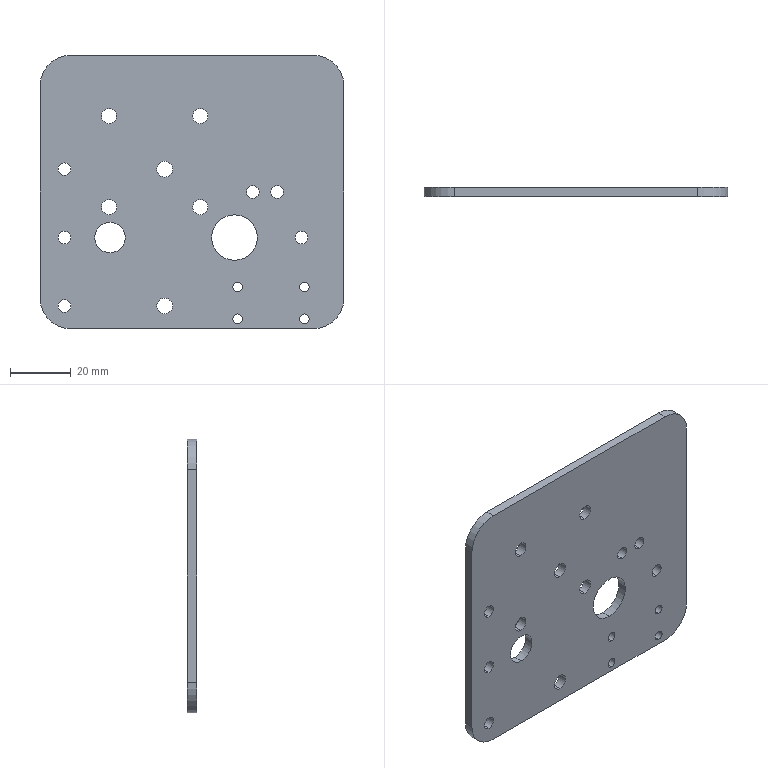Part | SolidWorks | features BaseBody 1 | 1 solid | 46 faces | box 100 x 3 x 90 mm | volume 25268 mm3 | cylinder 40 | plane 6 | commonest cylinder face diameters 4.2 x12 3.2 x8 5 x8 5.2 x4 20 x4 10 x2
STEP:
#1=CARTESIAN_POINT('',(28.,0.,12.9));
#2=VERTEX_POINT('',#1);
#3=CARTESIAN_POINT('',(28.,0.,17.1));
#4=VERTEX_POINT('',#3);
#5=CARTESIAN_POINT('',(28.,0.,15.));
#6=DIRECTION('',(0.,1.,0.));
#7=DIRECTION('',(0.,0.,1.));
#8=AXIS2_PLACEMENT_3D('',#5,#6,#7);
#9=CIRCLE('',#8,2.1);
#10=EDGE_CURVE('',#2,#4,#9,.T.);
#11=ORIENTED_EDGE('',*,*,#10,.F.);
#12=CARTESIAN_POINT('',(28.,3.,12.9));
#13=VERTEX_POINT('',#12);
#14=CARTESIAN_POINT('',(28.,0.,12.9));
#15=DIRECTION('',(0.,1.,0.));
#16=VECTOR('',#15,1000.);
#17=LINE('',#14,#16);
#18=EDGE_CURVE('',#2,#13,#17,.T.);
#19=ORIENTED_EDGE('',*,*,#18,.T.);
#20=CARTESIAN_POINT('',(28.,3.,17.1));
#21=VERTEX_POINT('',#20);
#22=CARTESIAN_POINT('',(28.,3.,15.));
#23=DIRECTION('',(0.,-1.,0.));
#24=DIRECTION('',(0.,0.,1.));
#25=AXIS2_PLACEMENT_3D('',#22,#23,#24);
#26=CIRCLE('',#25,2.1);
#27=EDGE_CURVE('',#21,#13,#26,.T.);
#28=ORIENTED_EDGE('',*,*,#27,.F.);
#29=CARTESIAN_POINT('',(28.,0.,17.1));
#30=DIRECTION('',(0.,1.,0.));
#31=VECTOR('',#30,1000.);
#32=LINE('',#29,#31);
#33=EDGE_CURVE('',#4,#21,#32,.T.);
#34=ORIENTED_EDGE('',*,*,#33,.F.);
#35=EDGE_LOOP('',(#11,#19,#28,#34));
#36=FACE_OUTER_BOUND('',#35,.T.);
#37=CARTESIAN_POINT('',(28.,0.,15.));
#38=DIRECTION('',(0.,1.,0.));
#39=DIRECTION('',(0.,0.,1.));
#40=AXIS2_PLACEMENT_3D('',#37,#38,#39);
#41=CYLINDRICAL_SURFACE('',#40,2.1);
#42=ADVANCED_FACE('',(#36),#41,.F.);
#43=CARTESIAN_POINT('',(20.,0.,12.9));
#44=VERTEX_POINT('',#43);
#45=CARTESIAN_POINT('',(20.,0.,17.1));
#46=VERTEX_POINT('',#45);
#47=CARTESIAN_POINT('',(20.,0.,15.));
#48=DIRECTION('',(0.,1.,0.));
#49=DIRECTION('',(0.,0.,1.));
#50=AXIS2_PLACEMENT_3D('',#47,#48,#49);
#51=CIRCLE('',#50,2.1);
#52=EDGE_CURVE('',#44,#46,#51,.T.);
#53=ORIENTED_EDGE('',*,*,#52,.F.);
#54=CARTESIAN_POINT('',(20.,3.,12.9));
#55=VERTEX_POINT('',#54);
#56=CARTESIAN_POINT('',(20.,0.,12.9));
#57=DIRECTION('',(0.,1.,0.));
#58=VECTOR('',#57,1000.);
#59=LINE('',#56,#58);
#60=EDGE_CURVE('',#44,#55,#59,.T.);
#61=ORIENTED_EDGE('',*,*,#60,.T.);
#62=CARTESIAN_POINT('',(20.,3.,17.1));
#63=VERTEX_POINT('',#62);
#64=CARTESIAN_POINT('',(20.,3.,15.));
#65=DIRECTION('',(0.,-1.,0.));
#66=DIRECTION('',(0.,0.,1.));
#67=AXIS2_PLACEMENT_3D('',#64,#65,#66);
#68=CIRCLE('',#67,2.1);
#69=EDGE_CURVE('',#63,#55,#68,.T.);
#70=ORIENTED_EDGE('',*,*,#69,.F.);
#71=CARTESIAN_POINT('',(20.,0.,17.1));
#72=DIRECTION('',(0.,1.,0.));
#73=VECTOR('',#72,1000.);
#74=LINE('',#71,#73);
#75=EDGE_CURVE('',#46,#63,#74,.T.);
#76=ORIENTED_EDGE('',*,*,#75,.F.);
#77=EDGE_LOOP('',(#53,#61,#70,#76));
#78=FACE_OUTER_BOUND('',#77,.T.);
#79=CARTESIAN_POINT('',(20.,0.,15.));
#80=DIRECTION('',(0.,1.,0.));
#81=DIRECTION('',(0.,0.,1.));
#82=AXIS2_PLACEMENT_3D('',#79,#80,#81);
#83=CYLINDRICAL_SURFACE('',#82,2.1);
#84=ADVANCED_FACE('',(#78),#83,.F.);
#85=CARTESIAN_POINT('',(-9.,0.,19.9));
#86=VERTEX_POINT('',#85);
#87=CARTESIAN_POINT('',(-9.,0.,25.1));
#88=VERTEX_POINT('',#87);
#89=CARTESIAN_POINT('',(-9.,0.,22.5));
#90=DIRECTION('',(0.,1.,0.));
#91=DIRECTION('',(0.,0.,1.));
#92=AXIS2_PLACEMENT_3D('',#89,#90,#91);
#93=CIRCLE('',#92,2.6);
#94=EDGE_CURVE('',#86,#88,#93,.T.);
#95=ORIENTED_EDGE('',*,*,#94,.F.);
#96=CARTESIAN_POINT('',(-9.,3.,19.9));
#97=VERTEX_POINT('',#96);
#98=CARTESIAN_POINT('',(-9.,0.,19.9));
#99=DIRECTION('',(0.,1.,0.));
#100=VECTOR('',#99,1000.);
#101=LINE('',#98,#100);
#102=EDGE_CURVE('',#86,#97,#101,.T.);
#103=ORIENTED_EDGE('',*,*,#102,.T.);
#104=CARTESIAN_POINT('',(-9.,3.,25.1));
#105=VERTEX_POINT('',#104);
#106=CARTESIAN_POINT('',(-9.,3.,22.5));
#107=DIRECTION('',(0.,-1.,0.));
#108=DIRECTION('',(0.,0.,1.));
#109=AXIS2_PLACEMENT_3D('',#106,#107,#108);
#110=CIRCLE('',#109,2.6);
#111=EDGE_CURVE('',#105,#97,#110,.T.);
#112=ORIENTED_EDGE('',*,*,#111,.F.);
#113=CARTESIAN_POINT('',(-9.,0.,25.1));
#114=DIRECTION('',(0.,1.,0.));
#115=VECTOR('',#114,1000.);
#116=LINE('',#113,#115);
#117=EDGE_CURVE('',#88,#105,#116,.T.);
#118=ORIENTED_EDGE('',*,*,#117,.F.);
#119=EDGE_LOOP('',(#95,#103,#112,#118));
#120=FACE_OUTER_BOUND('',#119,.T.);
#121=CARTESIAN_POINT('',(-9.,0.,22.5));
#122=DIRECTION('',(0.,1.,0.));
#123=DIRECTION('',(0.,0.,1.));
#124=AXIS2_PLACEMENT_3D('',#121,#122,#123);
#125=CYLINDRICAL_SURFACE('',#124,2.6);
#126=ADVANCED_FACE('',(#120),#125,.F.);
#127=CARTESIAN_POINT('',(-9.,0.,-25.1));
#128=VERTEX_POINT('',#127);
#129=CARTESIAN_POINT('',(-9.,0.,-19.9));
#130=VERTEX_POINT('',#129);
#131=CARTESIAN_POINT('',(-9.,0.,-22.5));
#132=DIRECTION('',(0.,1.,0.));
#133=DIRECTION('',(0.,0.,1.));
#134=AXIS2_PLACEMENT_3D('',#131,#132,#133);
#135=CIRCLE('',#134,2.6);
#136=EDGE_CURVE('',#128,#130,#135,.T.);
#137=ORIENTED_EDGE('',*,*,#136,.F.);
#138=CARTESIAN_POINT('',(-9.,3.,-25.1));
#139=VERTEX_POINT('',#138);
#140=CARTESIAN_POINT('',(-9.,0.,-25.1));
#141=DIRECTION('',(0.,1.,0.));
#142=VECTOR('',#141,1000.);
#143=LINE('',#140,#142);
#144=EDGE_CURVE('',#128,#139,#143,.T.);
#145=ORIENTED_EDGE('',*,*,#144,.T.);
#146=CARTESIAN_POINT('',(-9.,3.,-19.9));
#147=VERTEX_POINT('',#146);
#148=CARTESIAN_POINT('',(-9.,3.,-22.5));
#149=DIRECTION('',(0.,-1.,0.));
#150=DIRECTION('',(0.,0.,1.));
#151=AXIS2_PLACEMENT_3D('',#148,#149,#150);
#152=CIRCLE('',#151,2.6);
#153=EDGE_CURVE('',#147,#139,#152,.T.);
#154=ORIENTED_EDGE('',*,*,#153,.F.);
#155=CARTESIAN_POINT('',(-9.,0.,-19.9));
#156=DIRECTION('',(0.,1.,0.));
#157=VECTOR('',#156,1000.);
#158=LINE('',#155,#157);
#159=EDGE_CURVE('',#130,#147,#158,.T.);
#160=ORIENTED_EDGE('',*,*,#159,.F.);
#161=EDGE_LOOP('',(#137,#145,#154,#160));
#162=FACE_OUTER_BOUND('',#161,.T.);
#163=CARTESIAN_POINT('',(-9.,0.,-22.5));
#164=DIRECTION('',(0.,1.,0.));
#165=DIRECTION('',(0.,0.,1.));
#166=AXIS2_PLACEMENT_3D('',#163,#164,#165);
#167=CYLINDRICAL_SURFACE('',#166,2.6);
#168=ADVANCED_FACE('',(#162),#167,.F.);
#169=CARTESIAN_POINT('',(-42.,0.,-2.1));
#170=VERTEX_POINT('',#169);
#171=CARTESIAN_POINT('',(-42.,0.,2.1));
#172=VERTEX_POINT('',#171);
#173=CARTESIAN_POINT('',(-42.,0.,0.));
#174=DIRECTION('',(0.,1.,0.));
#175=DIRECTION('',(0.,0.,1.));
#176=AXIS2_PLACEMENT_3D('',#173,#174,#175);
#177=CIRCLE('',#176,2.1);
#178=EDGE_CURVE('',#170,#172,#177,.T.);
#179=ORIENTED_EDGE('',*,*,#178,.F.);
#180=CARTESIAN_POINT('',(-42.,3.,-2.1));
#181=VERTEX_POINT('',#180);
#182=CARTESIAN_POINT('',(-42.,0.,-2.1));
#183=DIRECTION('',(0.,1.,0.));
#184=VECTOR('',#183,1000.);
#185=LINE('',#182,#184);
#186=EDGE_CURVE('',#170,#181,#185,.T.);
#187=ORIENTED_EDGE('',*,*,#186,.T.);
#188=CARTESIAN_POINT('',(-42.,3.,2.1));
#189=VERTEX_POINT('',#188);
#190=CARTESIAN_POINT('',(-42.,3.,0.));
#191=DIRECTION('',(0.,-1.,0.));
#192=DIRECTION('',(0.,0.,1.));
#193=AXIS2_PLACEMENT_3D('',#190,#191,#192);
#194=CIRCLE('',#193,2.1);
#195=EDGE_CURVE('',#189,#181,#194,.T.);
#196=ORIENTED_EDGE('',*,*,#195,.F.);
#197=CARTESIAN_POINT('',(-42.,0.,2.1));
#198=DIRECTION('',(0.,1.,0.));
#199=VECTOR('',#198,1000.);
#200=LINE('',#197,#199);
#201=EDGE_CURVE('',#172,#189,#200,.T.);
#202=ORIENTED_EDGE('',*,*,#201,.F.);
#203=EDGE_LOOP('',(#179,#187,#196,#202));
#204=FACE_OUTER_BOUND('',#203,.T.);
#205=CARTESIAN_POINT('',(-42.,0.,0.));
#206=DIRECTION('',(0.,1.,0.));
#207=DIRECTION('',(0.,0.,1.));
#208=AXIS2_PLACEMENT_3D('',#205,#206,#207);
#209=CYLINDRICAL_SURFACE('',#208,2.1);
#210=ADVANCED_FACE('',(#204),#209,.F.);
#211=CARTESIAN_POINT('',(-27.,0.,-5.));
#212=VERTEX_POINT('',#211);
#213=CARTESIAN_POINT('',(-27.,0.,5.));
#214=VERTEX_POINT('',#213);
#215=CARTESIAN_POINT('',(-27.,0.,0.));
#216=DIRECTION('',(0.,1.,0.));
#217=DIRECTION('',(0.,0.,1.));
#218=AXIS2_PLACEMENT_3D('',#215,#216,#217);
#219=CIRCLE('',#218,5.);
#220=EDGE_CURVE('',#212,#214,#219,.T.);
#221=ORIENTED_EDGE('',*,*,#220,.F.);
#222=CARTESIAN_POINT('',(-27.,3.,-5.));
#223=VERTEX_POINT('',#222);
#224=CARTESIAN_POINT('',(-27.,0.,-5.));
#225=DIRECTION('',(0.,1.,0.));
#226=VECTOR('',#225,1000.);
#227=LINE('',#224,#226);
#228=EDGE_CURVE('',#212,#223,#227,.T.);
#229=ORIENTED_EDGE('',*,*,#228,.T.);
#230=CARTESIAN_POINT('',(-27.,3.,5.));
#231=VERTEX_POINT('',#230);
#232=CARTESIAN_POINT('',(-27.,3.,0.));
#233=DIRECTION('',(0.,-1.,0.));
#234=DIRECTION('',(0.,0.,1.));
#235=AXIS2_PLACEMENT_3D('',#232,#233,#234);
#236=CIRCLE('',#235,5.);
#237=EDGE_CURVE('',#231,#223,#236,.T.);
#238=ORIENTED_EDGE('',*,*,#237,.F.);
#239=CARTESIAN_POINT('',(-27.,0.,5.));
#240=DIRECTION('',(0.,1.,0.));
#241=VECTOR('',#240,1000.);
#242=LINE('',#239,#241);
#243=EDGE_CURVE('',#214,#231,#242,.T.);
#244=ORIENTED_EDGE('',*,*,#243,.F.);
#245=EDGE_LOOP('',(#221,#229,#238,#244));
#246=FACE_OUTER_BOUND('',#245,.T.);
#247=CARTESIAN_POINT('',(-27.,0.,0.));
#248=DIRECTION('',(0.,1.,0.));
#249=DIRECTION('',(0.,0.,1.));
#250=AXIS2_PLACEMENT_3D('',#247,#248,#249);
#251=CYLINDRICAL_SURFACE('',#250,5.);
#252=ADVANCED_FACE('',(#246),#251,.F.);
#253=CARTESIAN_POINT('',(14.,0.,-7.5));
#254=VERTEX_POINT('',#253);
#255=CARTESIAN_POINT('',(14.,0.,7.5));
#256=VERTEX_POINT('',#255);
#257=CARTESIAN_POINT('',(14.,0.,0.));
#258=DIRECTION('',(0.,1.,0.));
#259=DIRECTION('',(0.,0.,1.));
#260=AXIS2_PLACEMENT_3D('',#257,#258,#259);
#261=CIRCLE('',#260,7.5);
#262=EDGE_CURVE('',#254,#256,#261,.T.);
#263=ORIENTED_EDGE('',*,*,#262,.F.);
#264=CARTESIAN_POINT('',(14.,3.,-7.5));
#265=VERTEX_POINT('',#264);
#266=CARTESIAN_POINT('',(14.,0.,-7.5));
#267=DIRECTION('',(0.,1.,0.));
#268=VECTOR('',#267,1000.);
#269=LINE('',#266,#268);
#270=EDGE_CURVE('',#254,#265,#269,.T.);
#271=ORIENTED_EDGE('',*,*,#270,.T.);
#272=CARTESIAN_POINT('',(14.,3.,7.5));
#273=VERTEX_POINT('',#272);
#274=CARTESIAN_POINT('',(14.,3.,0.));
#275=DIRECTION('',(0.,-1.,0.));
#276=DIRECTION('',(0.,0.,1.));
#277=AXIS2_PLACEMENT_3D('',#274,#275,#276);
#278=CIRCLE('',#277,7.5);
#279=EDGE_CURVE('',#273,#265,#278,.T.);
#280=ORIENTED_EDGE('',*,*,#279,.F.);
#281=CARTESIAN_POINT('',(14.,0.,7.5));
#282=DIRECTION('',(0.,1.,0.));
#283=VECTOR('',#282,1000.);
#284=LINE('',#281,#283);
#285=EDGE_CURVE('',#256,#273,#284,.T.);
#286=ORIENTED_EDGE('',*,*,#285,.F.);
#287=EDGE_LOOP('',(#263,#271,#280,#286));
#288=FACE_OUTER_BOUND('',#287,.T.);
#289=CARTESIAN_POINT('',(14.,0.,0.));
#290=DIRECTION('',(0.,1.,0.));
#291=DIRECTION('',(0.,0.,1.));
#292=AXIS2_PLACEMENT_3D('',#289,#290,#291);
#293=CYLINDRICAL_SURFACE('',#292,7.5);
#294=ADVANCED_FACE('',(#288),#293,.F.);
#295=CARTESIAN_POINT('',(36.,0.,-2.1));
#296=VERTEX_POINT('',#295);
#297=CARTESIAN_POINT('',(36.,0.,2.1));
#298=VERTEX_POINT('',#297);
#299=CARTESIAN_POINT('',(36.,0.,0.));
#300=DIRECTION('',(0.,1.,0.));
#301=DIRECTION('',(0.,0.,1.));
#302=AXIS2_PLACEMENT_3D('',#299,#300,#301);
#303=CIRCLE('',#302,2.1);
#304=EDGE_CURVE('',#296,#298,#303,.T.);
#305=ORIENTED_EDGE('',*,*,#304,.F.);
#306=CARTESIAN_POINT('',(36.,3.,-2.1));
#307=VERTEX_POINT('',#306);
#308=CARTESIAN_POINT('',(36.,0.,-2.1));
#309=DIRECTION('',(0.,1.,0.));
#310=VECTOR('',#309,1000.);
#311=LINE('',#308,#310);
#312=EDGE_CURVE('',#296,#307,#311,.T.);
#313=ORIENTED_EDGE('',*,*,#312,.T.);
#314=CARTESIAN_POINT('',(36.,3.,2.1));
#315=VERTEX_POINT('',#314);
#316=CARTESIAN_POINT('',(36.,3.,0.));
#317=DIRECTION('',(0.,-1.,0.));
#318=DIRECTION('',(0.,0.,1.));
#319=AXIS2_PLACEMENT_3D('',#316,#317,#318);
#320=CIRCLE('',#319,2.1);
#321=EDGE_CURVE('',#315,#307,#320,.T.);
#322=ORIENTED_EDGE('',*,*,#321,.F.);
#323=CARTESIAN_POINT('',(36.,0.,2.1));
#324=DIRECTION('',(0.,1.,0.));
#325=VECTOR('',#324,1000.);
#326=LINE('',#323,#325);
#327=EDGE_CURVE('',#298,#315,#326,.T.);
#328=ORIENTED_EDGE('',*,*,#327,.F.);
#329=EDGE_LOOP('',(#305,#313,#322,#328));
#330=FACE_OUTER_BOUND('',#329,.T.);
#331=CARTESIAN_POINT('',(36.,0.,0.));
#332=DIRECTION('',(0.,1.,0.));
#333=DIRECTION('',(0.,0.,1.));
#334=AXIS2_PLACEMENT_3D('',#331,#332,#333);
#335=CYLINDRICAL_SURFACE('',#334,2.1);
#336=ADVANCED_FACE('',(#330),#335,.F.);
#337=CARTESIAN_POINT('',(-42.,0.,20.4));
#338=VERTEX_POINT('',#337);
#339=CARTESIAN_POINT('',(-42.,0.,24.6));
#340=VERTEX_POINT('',#339);
#341=CARTESIAN_POINT('',(-42.,0.,22.5));
#342=DIRECTION('',(0.,1.,0.));
#343=DIRECTION('',(0.,0.,1.));
#344=AXIS2_PLACEMENT_3D('',#341,#342,#343);
#345=CIRCLE('',#344,2.1);
#346=EDGE_CURVE('',#338,#340,#345,.T.);
#347=ORIENTED_EDGE('',*,*,#346,.F.);
#348=CARTESIAN_POINT('',(-42.,3.,20.4));
#349=VERTEX_POINT('',#348);
#350=CARTESIAN_POINT('',(-42.,0.,20.4));
#351=DIRECTION('',(0.,1.,0.));
#352=VECTOR('',#351,1000.);
#353=LINE('',#350,#352);
#354=EDGE_CURVE('',#338,#349,#353,.T.);
#355=ORIENTED_EDGE('',*,*,#354,.T.);
#356=CARTESIAN_POINT('',(-42.,3.,24.6));
#357=VERTEX_POINT('',#356);
#358=CARTESIAN_POINT('',(-42.,3.,22.5));
#359=DIRECTION('',(0.,-1.,0.));
#360=DIRECTION('',(0.,0.,1.));
#361=AXIS2_PLACEMENT_3D('',#358,#359,#360);
#362=CIRCLE('',#361,2.1);
#363=EDGE_CURVE('',#357,#349,#362,.T.);
#364=ORIENTED_EDGE('',*,*,#363,.F.);
#365=CARTESIAN_POINT('',(-42.,0.,24.6));
#366=DIRECTION('',(0.,1.,0.));
#367=VECTOR('',#366,1000.);
#368=LINE('',#365,#367);
#369=EDGE_CURVE('',#340,#357,#368,.T.);
#370=ORIENTED_EDGE('',*,*,#369,.F.);
#371=EDGE_LOOP('',(#347,#355,#364,#370));
#372=FACE_OUTER_BOUND('',#371,.T.);
#373=CARTESIAN_POINT('',(-42.,0.,22.5));
#374=DIRECTION('',(0.,1.,0.));
#375=DIRECTION('',(0.,0.,1.));
#376=AXIS2_PLACEMENT_3D('',#373,#374,#375);
#377=CYLINDRICAL_SURFACE('',#376,2.1);
#378=ADVANCED_FACE('',(#372),#377,.F.);
#379=CARTESIAN_POINT('',(-42.,0.,-24.6));
#380=VERTEX_POINT('',#379);
#381=CARTESIAN_POINT('',(-42.,0.,-20.4));
#382=VERTEX_POINT('',#381);
#383=CARTESIAN_POINT('',(-42.,0.,-22.5));
#384=DIRECTION('',(0.,1.,0.));
#385=DIRECTION('',(0.,0.,1.));
#386=AXIS2_PLACEMENT_3D('',#383,#384,#385);
#387=CIRCLE('',#386,2.1);
#388=EDGE_CURVE('',#380,#382,#387,.T.);
#389=ORIENTED_EDGE('',*,*,#388,.F.);
#390=CARTESIAN_POINT('',(-42.,3.,-24.6));
#391=VERTEX_POINT('',#390);
#392=CARTESIAN_POINT('',(-42.,0.,-24.6));
#393=DIRECTION('',(0.,1.,0.));
#394=VECTOR('',#393,1000.);
#395=LINE('',#392,#394);
#396=EDGE_CURVE('',#380,#391,#395,.T.);
#397=ORIENTED_EDGE('',*,*,#396,.T.);
#398=CARTESIAN_POINT('',(-42.,3.,-20.4));
#399=VERTEX_POINT('',#398);
#400=CARTESIAN_POINT('',(-42.,3.,-22.5));
#401=DIRECTION('',(0.,-1.,0.));
#402=DIRECTION('',(0.,0.,1.));
#403=AXIS2_PLACEMENT_3D('',#400,#401,#402);
#404=CIRCLE('',#403,2.1);
#405=EDGE_CURVE('',#399,#391,#404,.T.);
#406=ORIENTED_EDGE('',*,*,#405,.F.);
#407=CARTESIAN_POINT('',(-42.,0.,-20.4));
#408=DIRECTION('',(0.,1.,0.));
#409=VECTOR('',#408,1000.);
#410=LINE('',#407,#409);
#411=EDGE_CURVE('',#382,#399,#410,.T.);
#412=ORIENTED_EDGE('',*,*,#411,.F.);
#413=EDGE_LOOP('',(#389,#397,#406,#412));
#414=FACE_OUTER_BOUND('',#413,.T.);
#415=CARTESIAN_POINT('',(-42.,0.,-22.5));
#416=DIRECTION('',(0.,1.,0.));
#417=DIRECTION('',(0.,0.,1.));
#418=AXIS2_PLACEMENT_3D('',#415,#416,#417);
#419=CYLINDRICAL_SURFACE('',#418,2.1);
#420=ADVANCED_FACE('',(#414),#419,.F.);
#421=CARTESIAN_POINT('',(37.,0.,-28.35));
#422=VERTEX_POINT('',#421);
#423=CARTESIAN_POINT('',(37.,0.,-25.15));
#424=VERTEX_POINT('',#423);
#425=CARTESIAN_POINT('',(37.,0.,-26.75));
#426=DIRECTION('',(0.,1.,0.));
#427=DIRECTION('',(0.,0.,1.));
#428=AXIS2_PLACEMENT_3D('',#425,#426,#427);
#429=CIRCLE('',#428,1.6);
#430=EDGE_CURVE('',#422,#424,#429,.T.);
#431=ORIENTED_EDGE('',*,*,#430,.F.);
#432=CARTESIAN_POINT('',(37.,3.,-28.35));
#433=VERTEX_POINT('',#432);
#434=CARTESIAN_POINT('',(37.,0.,-28.35));
#435=DIRECTION('',(0.,1.,0.));
#436=VECTOR('',#435,1000.);
#437=LINE('',#434,#436);
#438=EDGE_CURVE('',#422,#433,#437,.T.);
#439=ORIENTED_EDGE('',*,*,#438,.T.);
#440=CARTESIAN_POINT('',(37.,3.,-25.15));
#441=VERTEX_POINT('',#440);
#442=CARTESIAN_POINT('',(37.,3.,-26.75));
#443=DIRECTION('',(0.,-1.,0.));
#444=DIRECTION('',(0.,0.,1.));
#445=AXIS2_PLACEMENT_3D('',#442,#443,#444);
#446=CIRCLE('',#445,1.6);
#447=EDGE_CURVE('',#441,#433,#446,.T.);
#448=ORIENTED_EDGE('',*,*,#447,.F.);
#449=CARTESIAN_POINT('',(37.,0.,-25.15));
#450=DIRECTION('',(0.,1.,0.));
#451=VECTOR('',#450,1000.);
#452=LINE('',#449,#451);
#453=EDGE_CURVE('',#424,#441,#452,.T.);
#454=ORIENTED_EDGE('',*,*,#453,.F.);
#455=EDGE_LOOP('',(#431,#439,#448,#454));
#456=FACE_OUTER_BOUND('',#455,.T.);
#457=CARTESIAN_POINT('',(37.,0.,-26.75));
#458=DIRECTION('',(0.,1.,0.));
#459=DIRECTION('',(0.,0.,1.));
#460=AXIS2_PLACEMENT_3D('',#457,#458,#459);
#461=CYLINDRICAL_SURFACE('',#460,1.6);
#462=ADVANCED_FACE('',(#456),#461,.F.);
#463=CARTESIAN_POINT('',(15.,0.,-28.35));
#464=VERTEX_POINT('',#463);
#465=CARTESIAN_POINT('',(15.,0.,-25.15));
#466=VERTEX_POINT('',#465);
#467=CARTESIAN_POINT('',(15.,0.,-26.75));
#468=DIRECTION('',(0.,1.,0.));
#469=DIRECTION('',(0.,0.,1.));
#470=AXIS2_PLACEMENT_3D('',#467,#468,#469);
#471=CIRCLE('',#470,1.6);
#472=EDGE_CURVE('',#464,#466,#471,.T.);
#473=ORIENTED_EDGE('',*,*,#472,.F.);
#474=CARTESIAN_POINT('',(15.,3.,-28.35));
#475=VERTEX_POINT('',#474);
#476=CARTESIAN_POINT('',(15.,0.,-28.35));
#477=DIRECTION('',(0.,1.,0.));
#478=VECTOR('',#477,1000.);
#479=LINE('',#476,#478);
#480=EDGE_CURVE('',#464,#475,#479,.T.);
#481=ORIENTED_EDGE('',*,*,#480,.T.);
#482=CARTESIAN_POINT('',(15.,3.,-25.15));
#483=VERTEX_POINT('',#482);
#484=CARTESIAN_POINT('',(15.,3.,-26.75));
#485=DIRECTION('',(0.,-1.,0.));
#486=DIRECTION('',(0.,0.,1.));
#487=AXIS2_PLACEMENT_3D('',#484,#485,#486);
#488=CIRCLE('',#487,1.6);
#489=EDGE_CURVE('',#483,#475,#488,.T.);
#490=ORIENTED_EDGE('',*,*,#489,.F.);
#491=CARTESIAN_POINT('',(15.,0.,-25.15));
#492=DIRECTION('',(0.,1.,0.));
#493=VECTOR('',#492,1000.);
#494=LINE('',#491,#493);
#495=EDGE_CURVE('',#466,#483,#494,.T.);
#496=ORIENTED_EDGE('',*,*,#495,.F.);
#497=EDGE_LOOP('',(#473,#481,#490,#496));
#498=FACE_OUTER_BOUND('',#497,.T.);
#499=CARTESIAN_POINT('',(15.,0.,-26.75));
#500=DIRECTION('',(0.,1.,0.));
#501=DIRECTION('',(0.,0.,1.));
#502=AXIS2_PLACEMENT_3D('',#499,#500,#501);
#503=CYLINDRICAL_SURFACE('',#502,1.6);
#504=ADVANCED_FACE('',(#498),#503,.F.);
#505=CARTESIAN_POINT('',(15.,0.,-17.85));
#506=VERTEX_POINT('',#505);
#507=CARTESIAN_POINT('',(15.,0.,-14.65));
#508=VERTEX_POINT('',#507);
#509=CARTESIAN_POINT('',(15.,0.,-16.25));
#510=DIRECTION('',(0.,1.,0.));
#511=DIRECTION('',(0.,0.,1.));
#512=AXIS2_PLACEMENT_3D('',#509,#510,#511);
#513=CIRCLE('',#512,1.6);
#514=EDGE_CURVE('',#506,#508,#513,.T.);
#515=ORIENTED_EDGE('',*,*,#514,.F.);
#516=CARTESIAN_POINT('',(15.,3.,-17.85));
#517=VERTEX_POINT('',#516);
#518=CARTESIAN_POINT('',(15.,0.,-17.85));
#519=DIRECTION('',(0.,1.,0.));
#520=VECTOR('',#519,1000.);
#521=LINE('',#518,#520);
#522=EDGE_CURVE('',#506,#517,#521,.T.);
#523=ORIENTED_EDGE('',*,*,#522,.T.);
#524=CARTESIAN_POINT('',(15.,3.,-14.65));
#525=VERTEX_POINT('',#524);
#526=CARTESIAN_POINT('',(15.,3.,-16.25));
#527=DIRECTION('',(0.,-1.,0.));
#528=DIRECTION('',(0.,0.,1.));
#529=AXIS2_PLACEMENT_3D('',#526,#527,#528);
#530=CIRCLE('',#529,1.6);
#531=EDGE_CURVE('',#525,#517,#530,.T.);
#532=ORIENTED_EDGE('',*,*,#531,.F.);
#533=CARTESIAN_POINT('',(15.,0.,-14.65));
#534=DIRECTION('',(0.,1.,0.));
#535=VECTOR('',#534,1000.);
#536=LINE('',#533,#535);
#537=EDGE_CURVE('',#508,#525,#536,.T.);
#538=ORIENTED_EDGE('',*,*,#537,.F.);
#539=EDGE_LOOP('',(#515,#523,#532,#538));
#540=FACE_OUTER_BOUND('',#539,.T.);
#541=CARTESIAN_POINT('',(15.,0.,-16.25));
#542=DIRECTION('',(0.,1.,0.));
#543=DIRECTION('',(0.,0.,1.));
#544=AXIS2_PLACEMENT_3D('',#541,#542,#543);
#545=CYLINDRICAL_SURFACE('',#544,1.6);
#546=ADVANCED_FACE('',(#540),#545,.F.);
#547=CARTESIAN_POINT('',(37.,0.,-17.85));
#548=VERTEX_POINT('',#547);
#549=CARTESIAN_POINT('',(37.,0.,-14.65));
#550=VERTEX_POINT('',#549);
#551=CARTESIAN_POINT('',(37.,0.,-16.25));
#552=DIRECTION('',(0.,1.,0.));
#553=DIRECTION('',(0.,0.,1.));
#554=AXIS2_PLACEMENT_3D('',#551,#552,#553);
#555=CIRCLE('',#554,1.6);
#556=EDGE_CURVE('',#548,#550,#555,.T.);
#557=ORIENTED_EDGE('',*,*,#556,.F.);
#558=CARTESIAN_POINT('',(37.,3.,-17.85));
#559=VERTEX_POINT('',#558);
#560=CARTESIAN_POINT('',(37.,0.,-17.85));
#561=DIRECTION('',(0.,1.,0.));
#562=VECTOR('',#561,1000.);
#563=LINE('',#560,#562);
#564=EDGE_CURVE('',#548,#559,#563,.T.);
#565=ORIENTED_EDGE('',*,*,#564,.T.);
#566=CARTESIAN_POINT('',(37.,3.,-14.65));
#567=VERTEX_POINT('',#566);
#568=CARTESIAN_POINT('',(37.,3.,-16.25));
#569=DIRECTION('',(0.,-1.,0.));
#570=DIRECTION('',(0.,0.,1.));
#571=AXIS2_PLACEMENT_3D('',#568,#569,#570);
#572=CIRCLE('',#571,1.6);
#573=EDGE_CURVE('',#567,#559,#572,.T.);
#574=ORIENTED_EDGE('',*,*,#573,.F.);
#575=CARTESIAN_POINT('',(37.,0.,-14.65));
#576=DIRECTION('',(0.,1.,0.));
#577=VECTOR('',#576,1000.);
#578=LINE('',#575,#577);
#579=EDGE_CURVE('',#550,#567,#578,.T.);
#580=ORIENTED_EDGE('',*,*,#579,.F.);
#581=EDGE_LOOP('',(#557,#565,#574,#580));
#582=FACE_OUTER_BOUND('',#581,.T.);
#583=CARTESIAN_POINT('',(37.,0.,-16.25));
#584=DIRECTION('',(0.,1.,0.));
#585=DIRECTION('',(0.,0.,1.));
#586=AXIS2_PLACEMENT_3D('',#583,#584,#585);
#587=CYLINDRICAL_SURFACE('',#586,1.6);
#588=ADVANCED_FACE('',(#582),#587,.F.);
#589=CARTESIAN_POINT('',(-27.3,0.,7.5));
#590=VERTEX_POINT('',#589);
#591=CARTESIAN_POINT('',(-27.3,0.,12.5));
#592=VERTEX_POINT('',#591);
#593=CARTESIAN_POINT('',(-27.3,0.,10.));
#594=DIRECTION('',(0.,1.,0.));
#595=DIRECTION('',(0.,0.,1.));
#596=AXIS2_PLACEMENT_3D('',#593,#594,#595);
#597=CIRCLE('',#596,2.5);
#598=EDGE_CURVE('',#590,#592,#597,.T.);
#599=ORIENTED_EDGE('',*,*,#598,.F.);
#600=CARTESIAN_POINT('',(-27.3,3.,7.5));
#601=VERTEX_POINT('',#600);
#602=CARTESIAN_POINT('',(-27.3,-7.,7.5));
#603=DIRECTION('',(0.,1.,0.));
#604=VECTOR('',#603,1000.);
#605=LINE('',#602,#604);
#606=EDGE_CURVE('',#590,#601,#605,.T.);
#607=ORIENTED_EDGE('',*,*,#606,.T.);
#608=CARTESIAN_POINT('',(-27.3,3.,12.5));
#609=VERTEX_POINT('',#608);
#610=CARTESIAN_POINT('',(-27.3,3.,10.));
#611=DIRECTION('',(0.,-1.,0.));
#612=DIRECTION('',(0.,0.,1.));
#613=AXIS2_PLACEMENT_3D('',#610,#611,#612);
#614=CIRCLE('',#613,2.5);
#615=EDGE_CURVE('',#609,#601,#614,.T.);
#616=ORIENTED_EDGE('',*,*,#615,.F.);
#617=CARTESIAN_POINT('',(-27.3,-7.,12.5));
#618=DIRECTION('',(0.,1.,0.));
#619=VECTOR('',#618,1000.);
#620=LINE('',#617,#619);
#621=EDGE_CURVE('',#592,#609,#620,.T.);
#622=ORIENTED_EDGE('',*,*,#621,.F.);
#623=EDGE_LOOP('',(#599,#607,#616,#622));
#624=FACE_OUTER_BOUND('',#623,.T.);
#625=CARTESIAN_POINT('',(-27.3,-7.,10.));
#626=DIRECTION('',(0.,1.,0.));
#627=DIRECTION('',(0.,0.,1.));
#628=AXIS2_PLACEMENT_3D('',#625,#626,#627);
#629=CYLINDRICAL_SURFACE('',#628,2.5);
#630=ADVANCED_FACE('',(#624),#629,.F.);
#631=CARTESIAN_POINT('',(2.7,0.,37.5));
#632=VERTEX_POINT('',#631);
#633=CARTESIAN_POINT('',(2.7,0.,42.5));
#634=VERTEX_POINT('',#633);
#635=CARTESIAN_POINT('',(2.7,0.,40.));
#636=DIRECTION('',(0.,1.,0.));
#637=DIRECTION('',(0.,0.,1.));
#638=AXIS2_PLACEMENT_3D('',#635,#636,#637);
#639=CIRCLE('',#638,2.5);
#640=EDGE_CURVE('',#632,#634,#639,.T.);
#641=ORIENTED_EDGE('',*,*,#640,.F.);
#642=CARTESIAN_POINT('',(2.7,3.,37.5));
#643=VERTEX_POINT('',#642);
#644=CARTESIAN_POINT('',(2.7,-7.,37.5));
#645=DIRECTION('',(0.,1.,0.));
#646=VECTOR('',#645,1000.);
#647=LINE('',#644,#646);
#648=EDGE_CURVE('',#632,#643,#647,.T.);
#649=ORIENTED_EDGE('',*,*,#648,.T.);
#650=CARTESIAN_POINT('',(2.7,3.,42.5));
#651=VERTEX_POINT('',#650);
#652=CARTESIAN_POINT('',(2.7,3.,40.));
#653=DIRECTION('',(0.,-1.,0.));
#654=DIRECTION('',(0.,0.,1.));
#655=AXIS2_PLACEMENT_3D('',#652,#653,#654);
#656=CIRCLE('',#655,2.5);
#657=EDGE_CURVE('',#651,#643,#656,.T.);
#658=ORIENTED_EDGE('',*,*,#657,.F.);
#659=CARTESIAN_POINT('',(2.7,-7.,42.5));
#660=DIRECTION('',(0.,1.,0.));
#661=VECTOR('',#660,1000.);
#662=LINE('',#659,#661);
#663=EDGE_CURVE('',#634,#651,#662,.T.);
#664=ORIENTED_EDGE('',*,*,#663,.F.);
#665=EDGE_LOOP('',(#641,#649,#658,#664));
#666=FACE_OUTER_BOUND('',#665,.T.);
#667=CARTESIAN_POINT('',(2.7,-7.,40.));
#668=DIRECTION('',(0.,1.,0.));
#669=DIRECTION('',(0.,0.,1.));
#670=AXIS2_PLACEMENT_3D('',#667,#668,#669);
#671=CYLINDRICAL_SURFACE('',#670,2.5);
#672=ADVANCED_FACE('',(#666),#671,.F.);
#673=CARTESIAN_POINT('',(-27.3,0.,37.5));
#674=VERTEX_POINT('',#673);
#675=CARTESIAN_POINT('',(-27.3,0.,42.5));
#676=VERTEX_POINT('',#675);
#677=CARTESIAN_POINT('',(-27.3,0.,40.));
#678=DIRECTION('',(0.,1.,0.));
#679=DIRECTION('',(0.,0.,1.));
#680=AXIS2_PLACEMENT_3D('',#677,#678,#679);
#681=CIRCLE('',#680,2.5);
#682=EDGE_CURVE('',#674,#676,#681,.T.);
#683=ORIENTED_EDGE('',*,*,#682,.F.);
#684=CARTESIAN_POINT('',(-27.3,3.,37.5));
#685=VERTEX_POINT('',#684);
#686=CARTESIAN_POINT('',(-27.3,-7.,37.5));
#687=DIRECTION('',(0.,1.,0.));
#688=VECTOR('',#687,1000.);
#689=LINE('',#686,#688);
#690=EDGE_CURVE('',#674,#685,#689,.T.);
#691=ORIENTED_EDGE('',*,*,#690,.T.);
#692=CARTESIAN_POINT('',(-27.3,3.,42.5));
#693=VERTEX_POINT('',#692);
#694=CARTESIAN_POINT('',(-27.3,3.,40.));
#695=DIRECTION('',(0.,-1.,0.));
#696=DIRECTION('',(0.,0.,1.));
#697=AXIS2_PLACEMENT_3D('',#694,#695,#696);
#698=CIRCLE('',#697,2.5);
#699=EDGE_CURVE('',#693,#685,#698,.T.);
#700=ORIENTED_EDGE('',*,*,#699,.F.);
#701=CARTESIAN_POINT('',(-27.3,-7.,42.5));
#702=DIRECTION('',(0.,1.,0.));
#703=VECTOR('',#702,1000.);
#704=LINE('',#701,#703);
#705=EDGE_CURVE('',#676,#693,#704,.T.);
#706=ORIENTED_EDGE('',*,*,#705,.F.);
#707=EDGE_LOOP('',(#683,#691,#700,#706));
#708=FACE_OUTER_BOUND('',#707,.T.);
#709=CARTESIAN_POINT('',(-27.3,-7.,40.));
#710=DIRECTION('',(0.,1.,0.));
#711=DIRECTION('',(0.,0.,1.));
#712=AXIS2_PLACEMENT_3D('',#709,#710,#711);
#713=CYLINDRICAL_SURFACE('',#712,2.5);
#714=ADVANCED_FACE('',(#708),#713,.F.);
#715=CARTESIAN_POINT('',(2.7,0.,7.5));
#716=VERTEX_POINT('',#715);
#717=CARTESIAN_POINT('',(2.7,0.,12.5));
#718=VERTEX_POINT('',#717);
#719=CARTESIAN_POINT('',(2.7,0.,10.));
#720=DIRECTION('',(0.,1.,0.));
#721=DIRECTION('',(0.,0.,1.));
#722=AXIS2_PLACEMENT_3D('',#719,#720,#721);
#723=CIRCLE('',#722,2.5);
#724=EDGE_CURVE('',#716,#718,#723,.T.);
#725=ORIENTED_EDGE('',*,*,#724,.F.);
#726=CARTESIAN_POINT('',(2.7,3.,7.5));
#727=VERTEX_POINT('',#726);
#728=CARTESIAN_POINT('',(2.7,-7.,7.5));
#729=DIRECTION('',(0.,1.,0.));
#730=VECTOR('',#729,1000.);
#731=LINE('',#728,#730);
#732=EDGE_CURVE('',#716,#727,#731,.T.);
#733=ORIENTED_EDGE('',*,*,#732,.T.);
#734=CARTESIAN_POINT('',(2.7,3.,12.5));
#735=VERTEX_POINT('',#734);
#736=CARTESIAN_POINT('',(2.7,3.,10.));
#737=DIRECTION('',(0.,-1.,0.));
#738=DIRECTION('',(0.,0.,1.));
#739=AXIS2_PLACEMENT_3D('',#736,#737,#738);
#740=CIRCLE('',#739,2.5);
#741=EDGE_CURVE('',#735,#727,#740,.T.);
#742=ORIENTED_EDGE('',*,*,#741,.F.);
#743=CARTESIAN_POINT('',(2.7,-7.,12.5));
#744=DIRECTION('',(0.,1.,0.));
#745=VECTOR('',#744,1000.);
#746=LINE('',#743,#745);
#747=EDGE_CURVE('',#718,#735,#746,.T.);
#748=ORIENTED_EDGE('',*,*,#747,.F.);
#749=EDGE_LOOP('',(#725,#733,#742,#748));
#750=FACE_OUTER_BOUND('',#749,.T.);
#751=CARTESIAN_POINT('',(2.7,-7.,10.));
#752=DIRECTION('',(0.,1.,0.));
#753=DIRECTION('',(0.,0.,1.));
#754=AXIS2_PLACEMENT_3D('',#751,#752,#753);
#755=CYLINDRICAL_SURFACE('',#754,2.5);
#756=ADVANCED_FACE('',(#750),#755,.F.);
#757=CARTESIAN_POINT('',(28.,0.,15.));
#758=DIRECTION('',(0.,1.,0.));
#759=DIRECTION('',(0.,0.,1.));
#760=AXIS2_PLACEMENT_3D('',#757,#758,#759);
#761=CIRCLE('',#760,2.1);
#762=EDGE_CURVE('',#4,#2,#761,.T.);
#763=ORIENTED_EDGE('',*,*,#762,.T.);
#764=ORIENTED_EDGE('',*,*,#10,.T.);
#765=EDGE_LOOP('',(#763,#764));
#766=FACE_BOUND('',#765,.T.);
#767=CARTESIAN_POINT('',(20.,0.,15.));
#768=DIRECTION('',(0.,1.,0.));
#769=DIRECTION('',(0.,0.,1.));
#770=AXIS2_PLACEMENT_3D('',#767,#768,#769);
#771=CIRCLE('',#770,2.1);
#772=EDGE_CURVE('',#46,#44,#771,.T.);
#773=ORIENTED_EDGE('',*,*,#772,.T.);
#774=ORIENTED_EDGE('',*,*,#52,.T.);
#775=EDGE_LOOP('',(#773,#774));
#776=FACE_BOUND('',#775,.T.);
#777=CARTESIAN_POINT('',(-9.,0.,22.5));
#778=DIRECTION('',(0.,1.,0.));
#779=DIRECTION('',(0.,0.,1.));
#780=AXIS2_PLACEMENT_3D('',#777,#778,#779);
#781=CIRCLE('',#780,2.6);
#782=EDGE_CURVE('',#88,#86,#781,.T.);
#783=ORIENTED_EDGE('',*,*,#782,.T.);
#784=ORIENTED_EDGE('',*,*,#94,.T.);
#785=EDGE_LOOP('',(#783,#784));
#786=FACE_BOUND('',#785,.T.);
#787=CARTESIAN_POINT('',(-9.,0.,-22.5));
#788=DIRECTION('',(0.,1.,0.));
#789=DIRECTION('',(0.,0.,1.));
#790=AXIS2_PLACEMENT_3D('',#787,#788,#789);
#791=CIRCLE('',#790,2.6);
#792=EDGE_CURVE('',#130,#128,#791,.T.);
#793=ORIENTED_EDGE('',*,*,#792,.T.);
#794=ORIENTED_EDGE('',*,*,#136,.T.);
#795=EDGE_LOOP('',(#793,#794));
#796=FACE_BOUND('',#795,.T.);
#797=CARTESIAN_POINT('',(-42.,0.,0.));
#798=DIRECTION('',(0.,1.,0.));
#799=DIRECTION('',(0.,0.,1.));
#800=AXIS2_PLACEMENT_3D('',#797,#798,#799);
#801=CIRCLE('',#800,2.1);
#802=EDGE_CURVE('',#172,#170,#801,.T.);
#803=ORIENTED_EDGE('',*,*,#802,.T.);
#804=ORIENTED_EDGE('',*,*,#178,.T.);
#805=EDGE_LOOP('',(#803,#804));
#806=FACE_BOUND('',#805,.T.);
#807=CARTESIAN_POINT('',(-27.,0.,0.));
#808=DIRECTION('',(0.,1.,0.));
#809=DIRECTION('',(0.,0.,1.));
#810=AXIS2_PLACEMENT_3D('',#807,#808,#809);
#811=CIRCLE('',#810,5.);
#812=EDGE_CURVE('',#214,#212,#811,.T.);
#813=ORIENTED_EDGE('',*,*,#812,.T.);
#814=ORIENTED_EDGE('',*,*,#220,.T.);
#815=EDGE_LOOP('',(#813,#814));
#816=FACE_BOUND('',#815,.T.);
#817=CARTESIAN_POINT('',(14.,0.,0.));
#818=DIRECTION('',(0.,1.,0.));
#819=DIRECTION('',(0.,0.,1.));
#820=AXIS2_PLACEMENT_3D('',#817,#818,#819);
#821=CIRCLE('',#820,7.5);
#822=EDGE_CURVE('',#256,#254,#821,.T.);
#823=ORIENTED_EDGE('',*,*,#822,.T.);
#824=ORIENTED_EDGE('',*,*,#262,.T.);
#825=EDGE_LOOP('',(#823,#824));
#826=FACE_BOUND('',#825,.T.);
#827=CARTESIAN_POINT('',(36.,0.,0.));
#828=DIRECTION('',(0.,1.,0.));
#829=DIRECTION('',(0.,0.,1.));
#830=AXIS2_PLACEMENT_3D('',#827,#828,#829);
#831=CIRCLE('',#830,2.1);
#832=EDGE_CURVE('',#298,#296,#831,.T.);
#833=ORIENTED_EDGE('',*,*,#832,.T.);
#834=ORIENTED_EDGE('',*,*,#304,.T.);
#835=EDGE_LOOP('',(#833,#834));
#836=FACE_BOUND('',#835,.T.);
#837=CARTESIAN_POINT('',(-42.,0.,22.5));
#838=DIRECTION('',(0.,1.,0.));
#839=DIRECTION('',(0.,0.,1.));
#840=AXIS2_PLACEMENT_3D('',#837,#838,#839);
#841=CIRCLE('',#840,2.1);
#842=EDGE_CURVE('',#340,#338,#841,.T.);
#843=ORIENTED_EDGE('',*,*,#842,.T.);
#844=ORIENTED_EDGE('',*,*,#346,.T.);
#845=EDGE_LOOP('',(#843,#844));
#846=FACE_BOUND('',#845,.T.);
#847=CARTESIAN_POINT('',(-42.,0.,-22.5));
#848=DIRECTION('',(0.,1.,0.));
#849=DIRECTION('',(0.,0.,1.));
#850=AXIS2_PLACEMENT_3D('',#847,#848,#849);
#851=CIRCLE('',#850,2.1);
#852=EDGE_CURVE('',#382,#380,#851,.T.);
#853=ORIENTED_EDGE('',*,*,#852,.T.);
#854=ORIENTED_EDGE('',*,*,#388,.T.);
#855=EDGE_LOOP('',(#853,#854));
#856=FACE_BOUND('',#855,.T.);
#857=CARTESIAN_POINT('',(37.,0.,-26.75));
#858=DIRECTION('',(0.,1.,0.));
#859=DIRECTION('',(0.,0.,1.));
#860=AXIS2_PLACEMENT_3D('',#857,#858,#859);
#861=CIRCLE('',#860,1.6);
#862=EDGE_CURVE('',#424,#422,#861,.T.);
#863=ORIENTED_EDGE('',*,*,#862,.T.);
#864=ORIENTED_EDGE('',*,*,#430,.T.);
#865=EDGE_LOOP('',(#863,#864));
#866=FACE_BOUND('',#865,.T.);
#867=CARTESIAN_POINT('',(15.,0.,-26.75));
#868=DIRECTION('',(0.,1.,0.));
#869=DIRECTION('',(0.,0.,1.));
#870=AXIS2_PLACEMENT_3D('',#867,#868,#869);
#871=CIRCLE('',#870,1.6);
#872=EDGE_CURVE('',#466,#464,#871,.T.);
#873=ORIENTED_EDGE('',*,*,#872,.T.);
#874=ORIENTED_EDGE('',*,*,#472,.T.);
#875=EDGE_LOOP('',(#873,#874));
#876=FACE_BOUND('',#875,.T.);
#877=CARTESIAN_POINT('',(15.,0.,-16.25));
#878=DIRECTION('',(0.,1.,0.));
#879=DIRECTION('',(0.,0.,1.));
#880=AXIS2_PLACEMENT_3D('',#877,#878,#879);
#881=CIRCLE('',#880,1.6);
#882=EDGE_CURVE('',#508,#506,#881,.T.);
#883=ORIENTED_EDGE('',*,*,#882,.T.);
#884=ORIENTED_EDGE('',*,*,#514,.T.);
#885=EDGE_LOOP('',(#883,#884));
#886=FACE_BOUND('',#885,.T.);
#887=CARTESIAN_POINT('',(37.,0.,-16.25));
#888=DIRECTION('',(0.,1.,0.));
#889=DIRECTION('',(0.,0.,1.));
#890=AXIS2_PLACEMENT_3D('',#887,#888,#889);
#891=CIRCLE('',#890,1.6);
#892=EDGE_CURVE('',#550,#548,#891,.T.);
#893=ORIENTED_EDGE('',*,*,#892,.T.);
#894=ORIENTED_EDGE('',*,*,#556,.T.);
#895=EDGE_LOOP('',(#893,#894));
#896=FACE_BOUND('',#895,.T.);
#897=CARTESIAN_POINT('',(-40.,0.,-30.));
#898=VERTEX_POINT('',#897);
#899=CARTESIAN_POINT('',(40.,0.,-30.));
#900=VERTEX_POINT('',#899);
#901=CARTESIAN_POINT('',(0.,0.,-30.));
#902=DIRECTION('',(1.,0.,0.));
#903=VECTOR('',#902,1000.);
#904=LINE('',#901,#903);
#905=EDGE_CURVE('',#898,#900,#904,.T.);
#906=ORIENTED_EDGE('',*,*,#905,.T.);
#907=CARTESIAN_POINT('',(50.,0.,-20.));
#908=VERTEX_POINT('',#907);
#909=CARTESIAN_POINT('',(40.,0.,-20.));
#910=DIRECTION('',(0.,-1.,0.));
#911=DIRECTION('',(0.,0.,-1.));
#912=AXIS2_PLACEMENT_3D('',#909,#910,#911);
#913=CIRCLE('',#912,10.);
#914=EDGE_CURVE('',#900,#908,#913,.T.);
#915=ORIENTED_EDGE('',*,*,#914,.T.);
#916=CARTESIAN_POINT('',(50.,0.,50.));
#917=VERTEX_POINT('',#916);
#918=CARTESIAN_POINT('',(50.,0.,0.));
#919=DIRECTION('',(0.,0.,1.));
#920=VECTOR('',#919,1000.);
#921=LINE('',#918,#920);
#922=EDGE_CURVE('',#908,#917,#921,.T.);
#923=ORIENTED_EDGE('',*,*,#922,.T.);
#924=CARTESIAN_POINT('',(40.,0.,60.));
#925=VERTEX_POINT('',#924);
#926=CARTESIAN_POINT('',(40.,0.,50.));
#927=DIRECTION('',(0.,-1.,0.));
#928=DIRECTION('',(0.,0.,1.));
#929=AXIS2_PLACEMENT_3D('',#926,#927,#928);
#930=CIRCLE('',#929,10.);
#931=EDGE_CURVE('',#917,#925,#930,.T.);
#932=ORIENTED_EDGE('',*,*,#931,.T.);
#933=CARTESIAN_POINT('',(-40.,0.,60.));
#934=VERTEX_POINT('',#933);
#935=CARTESIAN_POINT('',(0.,0.,60.));
#936=DIRECTION('',(-1.,0.,0.));
#937=VECTOR('',#936,1000.);
#938=LINE('',#935,#937);
#939=EDGE_CURVE('',#925,#934,#938,.T.);
#940=ORIENTED_EDGE('',*,*,#939,.T.);
#941=CARTESIAN_POINT('',(-50.,0.,50.));
#942=VERTEX_POINT('',#941);
#943=CARTESIAN_POINT('',(-40.,0.,50.));
#944=DIRECTION('',(0.,-1.,0.));
#945=DIRECTION('',(0.,0.,1.));
#946=AXIS2_PLACEMENT_3D('',#943,#944,#945);
#947=CIRCLE('',#946,10.);
#948=EDGE_CURVE('',#934,#942,#947,.T.);
#949=ORIENTED_EDGE('',*,*,#948,.T.);
#950=CARTESIAN_POINT('',(-50.,0.,-20.));
#951=VERTEX_POINT('',#950);
#952=CARTESIAN_POINT('',(-50.,0.,0.));
#953=DIRECTION('',(0.,0.,-1.));
#954=VECTOR('',#953,1000.);
#955=LINE('',#952,#954);
#956=EDGE_CURVE('',#942,#951,#955,.T.);
#957=ORIENTED_EDGE('',*,*,#956,.T.);
#958=CARTESIAN_POINT('',(-40.,0.,-20.));
#959=DIRECTION('',(0.,-1.,0.));
#960=DIRECTION('',(0.,0.,-1.));
#961=AXIS2_PLACEMENT_3D('',#958,#959,#960);
#962=CIRCLE('',#961,10.);
#963=EDGE_CURVE('',#951,#898,#962,.T.);
#964=ORIENTED_EDGE('',*,*,#963,.T.);
#965=EDGE_LOOP('',(#906,#915,#923,#932,#940,#949,#957,#964));
#966=FACE_OUTER_BOUND('',#965,.T.);
#967=CARTESIAN_POINT('',(-27.3,0.,10.));
#968=DIRECTION('',(0.,1.,0.));
#969=DIRECTION('',(0.,0.,1.));
#970=AXIS2_PLACEMENT_3D('',#967,#968,#969);
#971=CIRCLE('',#970,2.5);
#972=EDGE_CURVE('',#592,#590,#971,.T.);
#973=ORIENTED_EDGE('',*,*,#972,.T.);
#974=ORIENTED_EDGE('',*,*,#598,.T.);
#975=EDGE_LOOP('',(#973,#974));
#976=FACE_BOUND('',#975,.T.);
#977=CARTESIAN_POINT('',(2.7,0.,40.));
#978=DIRECTION('',(0.,1.,0.));
#979=DIRECTION('',(0.,0.,1.));
#980=AXIS2_PLACEMENT_3D('',#977,#978,#979);
#981=CIRCLE('',#980,2.5);
#982=EDGE_CURVE('',#634,#632,#981,.T.);
#983=ORIENTED_EDGE('',*,*,#982,.T.);
#984=ORIENTED_EDGE('',*,*,#640,.T.);
#985=EDGE_LOOP('',(#983,#984));
#986=FACE_BOUND('',#985,.T.);
#987=CARTESIAN_POINT('',(-27.3,0.,40.));
#988=DIRECTION('',(0.,1.,0.));
#989=DIRECTION('',(0.,0.,1.));
#990=AXIS2_PLACEMENT_3D('',#987,#988,#989);
#991=CIRCLE('',#990,2.5);
#992=EDGE_CURVE('',#676,#674,#991,.T.);
#993=ORIENTED_EDGE('',*,*,#992,.T.);
#994=ORIENTED_EDGE('',*,*,#682,.T.);
#995=EDGE_LOOP('',(#993,#994));
#996=FACE_BOUND('',#995,.T.);
#997=CARTESIAN_POINT('',(2.7,0.,10.));
#998=DIRECTION('',(0.,1.,0.));
#999=DIRECTION('',(0.,0.,1.));
#1000=AXIS2_PLACEMENT_3D('',#997,#998,#999);
#1001=CIRCLE('',#1000,2.5);
#1002=EDGE_CURVE('',#718,#716,#1001,.T.);
#1003=ORIENTED_EDGE('',*,*,#1002,.T.);
#1004=ORIENTED_EDGE('',*,*,#724,.T.);
#1005=EDGE_LOOP('',(#1003,#1004));
#1006=FACE_BOUND('',#1005,.T.);
#1007=CARTESIAN_POINT('',(0.,0.,0.));
#1008=DIRECTION('',(0.,-1.,0.));
#1009=DIRECTION('',(0.,0.,-1.));
#1010=AXIS2_PLACEMENT_3D('',#1007,#1008,#1009);
#1011=PLANE('',#1010);
#1012=ADVANCED_FACE('',(#766,#776,#786,#796,#806,#816,#826,#836,#846,#856,#866,#876,#886,#896,#966,#976,#986,#996,#1006),#1011,.T.);
#1013=ORIENTED_EDGE('',*,*,#18,.F.);
#1014=ORIENTED_EDGE('',*,*,#762,.F.);
#1015=ORIENTED_EDGE('',*,*,#33,.T.);
#1016=CARTESIAN_POINT('',(28.,3.,15.));
#1017=DIRECTION('',(0.,-1.,0.));
#1018=DIRECTION('',(0.,0.,1.));
#1019=AXIS2_PLACEMENT_3D('',#1016,#1017,#1018);
#1020=CIRCLE('',#1019,2.1);
#1021=EDGE_CURVE('',#13,#21,#1020,.T.);
#1022=ORIENTED_EDGE('',*,*,#1021,.F.);
#1023=EDGE_LOOP('',(#1013,#1014,#1015,#1022));
#1024=FACE_OUTER_BOUND('',#1023,.T.);
#1025=CARTESIAN_POINT('',(28.,0.,15.));
#1026=DIRECTION('',(0.,1.,0.));
#1027=DIRECTION('',(0.,0.,1.));
#1028=AXIS2_PLACEMENT_3D('',#1025,#1026,#1027);
#1029=CYLINDRICAL_SURFACE('',#1028,2.1);
#1030=ADVANCED_FACE('',(#1024),#1029,.F.);
#1031=ORIENTED_EDGE('',*,*,#60,.F.);
#1032=ORIENTED_EDGE('',*,*,#772,.F.);
#1033=ORIENTED_EDGE('',*,*,#75,.T.);
#1034=CARTESIAN_POINT('',(20.,3.,15.));
#1035=DIRECTION('',(0.,-1.,0.));
#1036=DIRECTION('',(0.,0.,1.));
#1037=AXIS2_PLACEMENT_3D('',#1034,#1035,#1036);
#1038=CIRCLE('',#1037,2.1);
#1039=EDGE_CURVE('',#55,#63,#1038,.T.);
#1040=ORIENTED_EDGE('',*,*,#1039,.F.);
#1041=EDGE_LOOP('',(#1031,#1032,#1033,#1040));
#1042=FACE_OUTER_BOUND('',#1041,.T.);
#1043=CARTESIAN_POINT('',(20.,0.,15.));
#1044=DIRECTION('',(0.,1.,0.));
#1045=DIRECTION('',(0.,0.,1.));
#1046=AXIS2_PLACEMENT_3D('',#1043,#1044,#1045);
#1047=CYLINDRICAL_SURFACE('',#1046,2.1);
#1048=ADVANCED_FACE('',(#1042),#1047,.F.);
#1049=ORIENTED_EDGE('',*,*,#102,.F.);
#1050=ORIENTED_EDGE('',*,*,#782,.F.);
#1051=ORIENTED_EDGE('',*,*,#117,.T.);
#1052=CARTESIAN_POINT('',(-9.,3.,22.5));
#1053=DIRECTION('',(0.,-1.,0.));
#1054=DIRECTION('',(0.,0.,1.));
#1055=AXIS2_PLACEMENT_3D('',#1052,#1053,#1054);
#1056=CIRCLE('',#1055,2.6);
#1057=EDGE_CURVE('',#97,#105,#1056,.T.);
#1058=ORIENTED_EDGE('',*,*,#1057,.F.);
#1059=EDGE_LOOP('',(#1049,#1050,#1051,#1058));
#1060=FACE_OUTER_BOUND('',#1059,.T.);
#1061=CARTESIAN_POINT('',(-9.,0.,22.5));
#1062=DIRECTION('',(0.,1.,0.));
#1063=DIRECTION('',(0.,0.,1.));
#1064=AXIS2_PLACEMENT_3D('',#1061,#1062,#1063);
#1065=CYLINDRICAL_SURFACE('',#1064,2.6);
#1066=ADVANCED_FACE('',(#1060),#1065,.F.);
#1067=ORIENTED_EDGE('',*,*,#144,.F.);
#1068=ORIENTED_EDGE('',*,*,#792,.F.);
#1069=ORIENTED_EDGE('',*,*,#159,.T.);
#1070=CARTESIAN_POINT('',(-9.,3.,-22.5));
#1071=DIRECTION('',(0.,-1.,0.));
#1072=DIRECTION('',(0.,0.,1.));
#1073=AXIS2_PLACEMENT_3D('',#1070,#1071,#1072);
#1074=CIRCLE('',#1073,2.6);
#1075=EDGE_CURVE('',#139,#147,#1074,.T.);
#1076=ORIENTED_EDGE('',*,*,#1075,.F.);
#1077=EDGE_LOOP('',(#1067,#1068,#1069,#1076));
#1078=FACE_OUTER_BOUND('',#1077,.T.);
#1079=CARTESIAN_POINT('',(-9.,0.,-22.5));
#1080=DIRECTION('',(0.,1.,0.));
#1081=DIRECTION('',(0.,0.,1.));
#1082=AXIS2_PLACEMENT_3D('',#1079,#1080,#1081);
#1083=CYLINDRICAL_SURFACE('',#1082,2.6);
#1084=ADVANCED_FACE('',(#1078),#1083,.F.);
#1085=ORIENTED_EDGE('',*,*,#186,.F.);
#1086=ORIENTED_EDGE('',*,*,#802,.F.);
#1087=ORIENTED_EDGE('',*,*,#201,.T.);
#1088=CARTESIAN_POINT('',(-42.,3.,0.));
#1089=DIRECTION('',(0.,-1.,0.));
#1090=DIRECTION('',(0.,0.,1.));
#1091=AXIS2_PLACEMENT_3D('',#1088,#1089,#1090);
#1092=CIRCLE('',#1091,2.1);
#1093=EDGE_CURVE('',#181,#189,#1092,.T.);
#1094=ORIENTED_EDGE('',*,*,#1093,.F.);
#1095=EDGE_LOOP('',(#1085,#1086,#1087,#1094));
#1096=FACE_OUTER_BOUND('',#1095,.T.);
#1097=CARTESIAN_POINT('',(-42.,0.,0.));
#1098=DIRECTION('',(0.,1.,0.));
#1099=DIRECTION('',(0.,0.,1.));
#1100=AXIS2_PLACEMENT_3D('',#1097,#1098,#1099);
#1101=CYLINDRICAL_SURFACE('',#1100,2.1);
#1102=ADVANCED_FACE('',(#1096),#1101,.F.);
#1103=ORIENTED_EDGE('',*,*,#228,.F.);
#1104=ORIENTED_EDGE('',*,*,#812,.F.);
#1105=ORIENTED_EDGE('',*,*,#243,.T.);
#1106=CARTESIAN_POINT('',(-27.,3.,0.));
#1107=DIRECTION('',(0.,-1.,0.));
#1108=DIRECTION('',(0.,0.,1.));
#1109=AXIS2_PLACEMENT_3D('',#1106,#1107,#1108);
#1110=CIRCLE('',#1109,5.);
#1111=EDGE_CURVE('',#223,#231,#1110,.T.);
#1112=ORIENTED_EDGE('',*,*,#1111,.F.);
#1113=EDGE_LOOP('',(#1103,#1104,#1105,#1112));
#1114=FACE_OUTER_BOUND('',#1113,.T.);
#1115=CARTESIAN_POINT('',(-27.,0.,0.));
#1116=DIRECTION('',(0.,1.,0.));
#1117=DIRECTION('',(0.,0.,1.));
#1118=AXIS2_PLACEMENT_3D('',#1115,#1116,#1117);
#1119=CYLINDRICAL_SURFACE('',#1118,5.);
#1120=ADVANCED_FACE('',(#1114),#1119,.F.);
#1121=ORIENTED_EDGE('',*,*,#270,.F.);
#1122=ORIENTED_EDGE('',*,*,#822,.F.);
#1123=ORIENTED_EDGE('',*,*,#285,.T.);
#1124=CARTESIAN_POINT('',(14.,3.,0.));
#1125=DIRECTION('',(0.,-1.,0.));
#1126=DIRECTION('',(0.,0.,1.));
#1127=AXIS2_PLACEMENT_3D('',#1124,#1125,#1126);
#1128=CIRCLE('',#1127,7.5);
#1129=EDGE_CURVE('',#265,#273,#1128,.T.);
#1130=ORIENTED_EDGE('',*,*,#1129,.F.);
#1131=EDGE_LOOP('',(#1121,#1122,#1123,#1130));
#1132=FACE_OUTER_BOUND('',#1131,.T.);
#1133=CARTESIAN_POINT('',(14.,0.,0.));
#1134=DIRECTION('',(0.,1.,0.));
#1135=DIRECTION('',(0.,0.,1.));
#1136=AXIS2_PLACEMENT_3D('',#1133,#1134,#1135);
#1137=CYLINDRICAL_SURFACE('',#1136,7.5);
#1138=ADVANCED_FACE('',(#1132),#1137,.F.);
#1139=ORIENTED_EDGE('',*,*,#312,.F.);
#1140=ORIENTED_EDGE('',*,*,#832,.F.);
#1141=ORIENTED_EDGE('',*,*,#327,.T.);
#1142=CARTESIAN_POINT('',(36.,3.,0.));
#1143=DIRECTION('',(0.,-1.,0.));
#1144=DIRECTION('',(0.,0.,1.));
#1145=AXIS2_PLACEMENT_3D('',#1142,#1143,#1144);
#1146=CIRCLE('',#1145,2.1);
#1147=EDGE_CURVE('',#307,#315,#1146,.T.);
#1148=ORIENTED_EDGE('',*,*,#1147,.F.);
#1149=EDGE_LOOP('',(#1139,#1140,#1141,#1148));
#1150=FACE_OUTER_BOUND('',#1149,.T.);
#1151=CARTESIAN_POINT('',(36.,0.,0.));
#1152=DIRECTION('',(0.,1.,0.));
#1153=DIRECTION('',(0.,0.,1.));
#1154=AXIS2_PLACEMENT_3D('',#1151,#1152,#1153);
#1155=CYLINDRICAL_SURFACE('',#1154,2.1);
#1156=ADVANCED_FACE('',(#1150),#1155,.F.);
#1157=ORIENTED_EDGE('',*,*,#354,.F.);
#1158=ORIENTED_EDGE('',*,*,#842,.F.);
#1159=ORIENTED_EDGE('',*,*,#369,.T.);
#1160=CARTESIAN_POINT('',(-42.,3.,22.5));
#1161=DIRECTION('',(0.,-1.,0.));
#1162=DIRECTION('',(0.,0.,1.));
#1163=AXIS2_PLACEMENT_3D('',#1160,#1161,#1162);
#1164=CIRCLE('',#1163,2.1);
#1165=EDGE_CURVE('',#349,#357,#1164,.T.);
#1166=ORIENTED_EDGE('',*,*,#1165,.F.);
#1167=EDGE_LOOP('',(#1157,#1158,#1159,#1166));
#1168=FACE_OUTER_BOUND('',#1167,.T.);
#1169=CARTESIAN_POINT('',(-42.,0.,22.5));
#1170=DIRECTION('',(0.,1.,0.));
#1171=DIRECTION('',(0.,0.,1.));
#1172=AXIS2_PLACEMENT_3D('',#1169,#1170,#1171);
#1173=CYLINDRICAL_SURFACE('',#1172,2.1);
#1174=ADVANCED_FACE('',(#1168),#1173,.F.);
#1175=ORIENTED_EDGE('',*,*,#396,.F.);
#1176=ORIENTED_EDGE('',*,*,#852,.F.);
#1177=ORIENTED_EDGE('',*,*,#411,.T.);
#1178=CARTESIAN_POINT('',(-42.,3.,-22.5));
#1179=DIRECTION('',(0.,-1.,0.));
#1180=DIRECTION('',(0.,0.,1.));
#1181=AXIS2_PLACEMENT_3D('',#1178,#1179,#1180);
#1182=CIRCLE('',#1181,2.1);
#1183=EDGE_CURVE('',#391,#399,#1182,.T.);
#1184=ORIENTED_EDGE('',*,*,#1183,.F.);
#1185=EDGE_LOOP('',(#1175,#1176,#1177,#1184));
#1186=FACE_OUTER_BOUND('',#1185,.T.);
#1187=CARTESIAN_POINT('',(-42.,0.,-22.5));
#1188=DIRECTION('',(0.,1.,0.));
#1189=DIRECTION('',(0.,0.,1.));
#1190=AXIS2_PLACEMENT_3D('',#1187,#1188,#1189);
#1191=CYLINDRICAL_SURFACE('',#1190,2.1);
#1192=ADVANCED_FACE('',(#1186),#1191,.F.);
#1193=ORIENTED_EDGE('',*,*,#438,.F.);
#1194=ORIENTED_EDGE('',*,*,#862,.F.);
#1195=ORIENTED_EDGE('',*,*,#453,.T.);
#1196=CARTESIAN_POINT('',(37.,3.,-26.75));
#1197=DIRECTION('',(0.,-1.,0.));
#1198=DIRECTION('',(0.,0.,1.));
#1199=AXIS2_PLACEMENT_3D('',#1196,#1197,#1198);
#1200=CIRCLE('',#1199,1.6);
#1201=EDGE_CURVE('',#433,#441,#1200,.T.);
#1202=ORIENTED_EDGE('',*,*,#1201,.F.);
#1203=EDGE_LOOP('',(#1193,#1194,#1195,#1202));
#1204=FACE_OUTER_BOUND('',#1203,.T.);
#1205=CARTESIAN_POINT('',(37.,0.,-26.75));
#1206=DIRECTION('',(0.,1.,0.));
#1207=DIRECTION('',(0.,0.,1.));
#1208=AXIS2_PLACEMENT_3D('',#1205,#1206,#1207);
#1209=CYLINDRICAL_SURFACE('',#1208,1.6);
#1210=ADVANCED_FACE('',(#1204),#1209,.F.);
#1211=ORIENTED_EDGE('',*,*,#480,.F.);
#1212=ORIENTED_EDGE('',*,*,#872,.F.);
#1213=ORIENTED_EDGE('',*,*,#495,.T.);
#1214=CARTESIAN_POINT('',(15.,3.,-26.75));
#1215=DIRECTION('',(0.,-1.,0.));
#1216=DIRECTION('',(0.,0.,1.));
#1217=AXIS2_PLACEMENT_3D('',#1214,#1215,#1216);
#1218=CIRCLE('',#1217,1.6);
#1219=EDGE_CURVE('',#475,#483,#1218,.T.);
#1220=ORIENTED_EDGE('',*,*,#1219,.F.);
#1221=EDGE_LOOP('',(#1211,#1212,#1213,#1220));
#1222=FACE_OUTER_BOUND('',#1221,.T.);
#1223=CARTESIAN_POINT('',(15.,0.,-26.75));
#1224=DIRECTION('',(0.,1.,0.));
#1225=DIRECTION('',(0.,0.,1.));
#1226=AXIS2_PLACEMENT_3D('',#1223,#1224,#1225);
#1227=CYLINDRICAL_SURFACE('',#1226,1.6);
#1228=ADVANCED_FACE('',(#1222),#1227,.F.);
#1229=ORIENTED_EDGE('',*,*,#522,.F.);
#1230=ORIENTED_EDGE('',*,*,#882,.F.);
#1231=ORIENTED_EDGE('',*,*,#537,.T.);
#1232=CARTESIAN_POINT('',(15.,3.,-16.25));
#1233=DIRECTION('',(0.,-1.,0.));
#1234=DIRECTION('',(0.,0.,1.));
#1235=AXIS2_PLACEMENT_3D('',#1232,#1233,#1234);
#1236=CIRCLE('',#1235,1.6);
#1237=EDGE_CURVE('',#517,#525,#1236,.T.);
#1238=ORIENTED_EDGE('',*,*,#1237,.F.);
#1239=EDGE_LOOP('',(#1229,#1230,#1231,#1238));
#1240=FACE_OUTER_BOUND('',#1239,.T.);
#1241=CARTESIAN_POINT('',(15.,0.,-16.25));
#1242=DIRECTION('',(0.,1.,0.));
#1243=DIRECTION('',(0.,0.,1.));
#1244=AXIS2_PLACEMENT_3D('',#1241,#1242,#1243);
#1245=CYLINDRICAL_SURFACE('',#1244,1.6);
#1246=ADVANCED_FACE('',(#1240),#1245,.F.);
#1247=ORIENTED_EDGE('',*,*,#564,.F.);
#1248=ORIENTED_EDGE('',*,*,#892,.F.);
#1249=ORIENTED_EDGE('',*,*,#579,.T.);
#1250=CARTESIAN_POINT('',(37.,3.,-16.25));
#1251=DIRECTION('',(0.,-1.,0.));
#1252=DIRECTION('',(0.,0.,1.));
#1253=AXIS2_PLACEMENT_3D('',#1250,#1251,#1252);
#1254=CIRCLE('',#1253,1.6);
#1255=EDGE_CURVE('',#559,#567,#1254,.T.);
#1256=ORIENTED_EDGE('',*,*,#1255,.F.);
#1257=EDGE_LOOP('',(#1247,#1248,#1249,#1256));
#1258=FACE_OUTER_BOUND('',#1257,.T.);
#1259=CARTESIAN_POINT('',(37.,0.,-16.25));
#1260=DIRECTION('',(0.,1.,0.));
#1261=DIRECTION('',(0.,0.,1.));
#1262=AXIS2_PLACEMENT_3D('',#1259,#1260,#1261);
#1263=CYLINDRICAL_SURFACE('',#1262,1.6);
#1264=ADVANCED_FACE('',(#1258),#1263,.F.);
#1265=ORIENTED_EDGE('',*,*,#914,.F.);
#1266=CARTESIAN_POINT('',(40.,3.,-30.));
#1267=VERTEX_POINT('',#1266);
#1268=CARTESIAN_POINT('',(40.,3.,-30.));
#1269=DIRECTION('',(0.,1.,0.));
#1270=VECTOR('',#1269,1000.);
#1271=LINE('',#1268,#1270);
#1272=EDGE_CURVE('',#900,#1267,#1271,.T.);
#1273=ORIENTED_EDGE('',*,*,#1272,.T.);
#1274=CARTESIAN_POINT('',(50.,3.,-20.));
#1275=VERTEX_POINT('',#1274);
#1276=CARTESIAN_POINT('',(40.,3.,-20.));
#1277=DIRECTION('',(0.,-1.,0.));
#1278=DIRECTION('',(0.,0.,-1.));
#1279=AXIS2_PLACEMENT_3D('',#1276,#1277,#1278);
#1280=CIRCLE('',#1279,10.);
#1281=EDGE_CURVE('',#1267,#1275,#1280,.T.);
#1282=ORIENTED_EDGE('',*,*,#1281,.T.);
#1283=CARTESIAN_POINT('',(50.,3.,-20.));
#1284=DIRECTION('',(0.,-1.,0.));
#1285=VECTOR('',#1284,1000.);
#1286=LINE('',#1283,#1285);
#1287=EDGE_CURVE('',#1275,#908,#1286,.T.);
#1288=ORIENTED_EDGE('',*,*,#1287,.T.);
#1289=EDGE_LOOP('',(#1265,#1273,#1282,#1288));
#1290=FACE_OUTER_BOUND('',#1289,.T.);
#1291=CARTESIAN_POINT('',(40.,3.,-20.));
#1292=DIRECTION('',(0.,-1.,0.));
#1293=DIRECTION('',(0.,0.,-1.));
#1294=AXIS2_PLACEMENT_3D('',#1291,#1292,#1293);
#1295=CYLINDRICAL_SURFACE('',#1294,10.);
#1296=ADVANCED_FACE('',(#1290),#1295,.T.);
#1297=CARTESIAN_POINT('',(-40.,3.,-30.));
#1298=VERTEX_POINT('',#1297);
#1299=CARTESIAN_POINT('',(-40.,3.,-30.));
#1300=DIRECTION('',(0.,-1.,0.));
#1301=VECTOR('',#1300,1000.);
#1302=LINE('',#1299,#1301);
#1303=EDGE_CURVE('',#1298,#898,#1302,.T.);
#1304=ORIENTED_EDGE('',*,*,#1303,.F.);
#1305=CARTESIAN_POINT('',(-50.,3.,-30.));
#1306=DIRECTION('',(-1.,0.,0.));
#1307=VECTOR('',#1306,1000.);
#1308=LINE('',#1305,#1307);
#1309=EDGE_CURVE('',#1267,#1298,#1308,.T.);
#1310=ORIENTED_EDGE('',*,*,#1309,.F.);
#1311=ORIENTED_EDGE('',*,*,#1272,.F.);
#1312=ORIENTED_EDGE('',*,*,#905,.F.);
#1313=EDGE_LOOP('',(#1304,#1310,#1311,#1312));
#1314=FACE_OUTER_BOUND('',#1313,.T.);
#1315=CARTESIAN_POINT('',(-50.,3.,-30.));
#1316=DIRECTION('',(0.,0.,1.));
#1317=DIRECTION('',(1.,0.,0.));
#1318=AXIS2_PLACEMENT_3D('',#1315,#1316,#1317);
#1319=PLANE('',#1318);
#1320=ADVANCED_FACE('',(#1314),#1319,.F.);
#1321=ORIENTED_EDGE('',*,*,#963,.F.);
#1322=CARTESIAN_POINT('',(-50.,3.,-20.));
#1323=VERTEX_POINT('',#1322);
#1324=CARTESIAN_POINT('',(-50.,3.,-20.));
#1325=DIRECTION('',(0.,1.,0.));
#1326=VECTOR('',#1325,1000.);
#1327=LINE('',#1324,#1326);
#1328=EDGE_CURVE('',#951,#1323,#1327,.T.);
#1329=ORIENTED_EDGE('',*,*,#1328,.T.);
#1330=CARTESIAN_POINT('',(-40.,3.,-20.));
#1331=DIRECTION('',(0.,-1.,0.));
#1332=DIRECTION('',(0.,0.,-1.));
#1333=AXIS2_PLACEMENT_3D('',#1330,#1331,#1332);
#1334=CIRCLE('',#1333,10.);
#1335=EDGE_CURVE('',#1323,#1298,#1334,.T.);
#1336=ORIENTED_EDGE('',*,*,#1335,.T.);
#1337=ORIENTED_EDGE('',*,*,#1303,.T.);
#1338=EDGE_LOOP('',(#1321,#1329,#1336,#1337));
#1339=FACE_OUTER_BOUND('',#1338,.T.);
#1340=CARTESIAN_POINT('',(-40.,3.,-20.));
#1341=DIRECTION('',(0.,-1.,0.));
#1342=DIRECTION('',(0.,0.,-1.));
#1343=AXIS2_PLACEMENT_3D('',#1340,#1341,#1342);
#1344=CYLINDRICAL_SURFACE('',#1343,10.);
#1345=ADVANCED_FACE('',(#1339),#1344,.T.);
#1346=CARTESIAN_POINT('',(-50.,3.,50.));
#1347=VERTEX_POINT('',#1346);
#1348=CARTESIAN_POINT('',(-50.,3.,50.));
#1349=DIRECTION('',(0.,-1.,0.));
#1350=VECTOR('',#1349,1000.);
#1351=LINE('',#1348,#1350);
#1352=EDGE_CURVE('',#1347,#942,#1351,.T.);
#1353=ORIENTED_EDGE('',*,*,#1352,.F.);
#1354=CARTESIAN_POINT('',(-50.,3.,30.));
#1355=DIRECTION('',(0.,0.,1.));
#1356=VECTOR('',#1355,1000.);
#1357=LINE('',#1354,#1356);
#1358=EDGE_CURVE('',#1323,#1347,#1357,.T.);
#1359=ORIENTED_EDGE('',*,*,#1358,.F.);
#1360=ORIENTED_EDGE('',*,*,#1328,.F.);
#1361=ORIENTED_EDGE('',*,*,#956,.F.);
#1362=EDGE_LOOP('',(#1353,#1359,#1360,#1361));
#1363=FACE_OUTER_BOUND('',#1362,.T.);
#1364=CARTESIAN_POINT('',(-50.,3.,30.));
#1365=DIRECTION('',(1.,0.,0.));
#1366=DIRECTION('',(0.,0.,-1.));
#1367=AXIS2_PLACEMENT_3D('',#1364,#1365,#1366);
#1368=PLANE('',#1367);
#1369=ADVANCED_FACE('',(#1363),#1368,.F.);
#1370=ORIENTED_EDGE('',*,*,#948,.F.);
#1371=CARTESIAN_POINT('',(-40.,3.,60.));
#1372=VERTEX_POINT('',#1371);
#1373=CARTESIAN_POINT('',(-40.,103.499,60.));
#1374=DIRECTION('',(0.,1.,0.));
#1375=VECTOR('',#1374,1000.);
#1376=LINE('',#1373,#1375);
#1377=EDGE_CURVE('',#934,#1372,#1376,.T.);
#1378=ORIENTED_EDGE('',*,*,#1377,.T.);
#1379=CARTESIAN_POINT('',(-40.,3.,50.));
#1380=DIRECTION('',(0.,-1.,0.));
#1381=DIRECTION('',(0.,0.,1.));
#1382=AXIS2_PLACEMENT_3D('',#1379,#1380,#1381);
#1383=CIRCLE('',#1382,10.);
#1384=EDGE_CURVE('',#1372,#1347,#1383,.T.);
#1385=ORIENTED_EDGE('',*,*,#1384,.T.);
#1386=ORIENTED_EDGE('',*,*,#1352,.T.);
#1387=EDGE_LOOP('',(#1370,#1378,#1385,#1386));
#1388=FACE_OUTER_BOUND('',#1387,.T.);
#1389=CARTESIAN_POINT('',(-40.,103.499,50.));
#1390=DIRECTION('',(0.,1.,0.));
#1391=DIRECTION('',(0.,0.,1.));
#1392=AXIS2_PLACEMENT_3D('',#1389,#1390,#1391);
#1393=CYLINDRICAL_SURFACE('',#1392,10.);
#1394=ADVANCED_FACE('',(#1388),#1393,.T.);
#1395=CARTESIAN_POINT('',(40.,3.,60.));
#1396=VERTEX_POINT('',#1395);
#1397=CARTESIAN_POINT('',(-50.,3.,60.));
#1398=DIRECTION('',(-1.,0.,0.));
#1399=VECTOR('',#1398,1000.);
#1400=LINE('',#1397,#1399);
#1401=EDGE_CURVE('',#1396,#1372,#1400,.T.);
#1402=ORIENTED_EDGE('',*,*,#1401,.T.);
#1403=ORIENTED_EDGE('',*,*,#1377,.F.);
#1404=ORIENTED_EDGE('',*,*,#939,.F.);
#1405=CARTESIAN_POINT('',(40.,103.499,60.));
#1406=DIRECTION('',(0.,1.,0.));
#1407=VECTOR('',#1406,1000.);
#1408=LINE('',#1405,#1407);
#1409=EDGE_CURVE('',#925,#1396,#1408,.T.);
#1410=ORIENTED_EDGE('',*,*,#1409,.T.);
#1411=EDGE_LOOP('',(#1402,#1403,#1404,#1410));
#1412=FACE_OUTER_BOUND('',#1411,.T.);
#1413=CARTESIAN_POINT('',(-50.,103.499,60.));
#1414=DIRECTION('',(0.,0.,1.));
#1415=DIRECTION('',(1.,0.,0.));
#1416=AXIS2_PLACEMENT_3D('',#1413,#1414,#1415);
#1417=PLANE('',#1416);
#1418=ADVANCED_FACE('',(#1412),#1417,.T.);
#1419=ORIENTED_EDGE('',*,*,#931,.F.);
#1420=CARTESIAN_POINT('',(50.,3.,50.));
#1421=VERTEX_POINT('',#1420);
#1422=CARTESIAN_POINT('',(50.,3.,50.));
#1423=DIRECTION('',(0.,1.,0.));
#1424=VECTOR('',#1423,1000.);
#1425=LINE('',#1422,#1424);
#1426=EDGE_CURVE('',#917,#1421,#1425,.T.);
#1427=ORIENTED_EDGE('',*,*,#1426,.T.);
#1428=CARTESIAN_POINT('',(40.,3.,50.));
#1429=DIRECTION('',(0.,-1.,0.));
#1430=DIRECTION('',(0.,0.,1.));
#1431=AXIS2_PLACEMENT_3D('',#1428,#1429,#1430);
#1432=CIRCLE('',#1431,10.);
#1433=EDGE_CURVE('',#1421,#1396,#1432,.T.);
#1434=ORIENTED_EDGE('',*,*,#1433,.T.);
#1435=ORIENTED_EDGE('',*,*,#1409,.F.);
#1436=EDGE_LOOP('',(#1419,#1427,#1434,#1435));
#1437=FACE_OUTER_BOUND('',#1436,.T.);
#1438=CARTESIAN_POINT('',(40.,3.,50.));
#1439=DIRECTION('',(0.,1.,0.));
#1440=DIRECTION('',(0.,0.,1.));
#1441=AXIS2_PLACEMENT_3D('',#1438,#1439,#1440);
#1442=CYLINDRICAL_SURFACE('',#1441,10.);
#1443=ADVANCED_FACE('',(#1437),#1442,.T.);
#1444=ORIENTED_EDGE('',*,*,#1426,.F.);
#1445=ORIENTED_EDGE('',*,*,#922,.F.);
#1446=ORIENTED_EDGE('',*,*,#1287,.F.);
#1447=CARTESIAN_POINT('',(50.,3.,30.));
#1448=DIRECTION('',(0.,0.,-1.));
#1449=VECTOR('',#1448,1000.);
#1450=LINE('',#1447,#1449);
#1451=EDGE_CURVE('',#1421,#1275,#1450,.T.);
#1452=ORIENTED_EDGE('',*,*,#1451,.F.);
#1453=EDGE_LOOP('',(#1444,#1445,#1446,#1452));
#1454=FACE_OUTER_BOUND('',#1453,.T.);
#1455=CARTESIAN_POINT('',(50.,3.,30.));
#1456=DIRECTION('',(-1.,0.,0.));
#1457=DIRECTION('',(0.,0.,1.));
#1458=AXIS2_PLACEMENT_3D('',#1455,#1456,#1457);
#1459=PLANE('',#1458);
#1460=ADVANCED_FACE('',(#1454),#1459,.F.);
#1461=ORIENTED_EDGE('',*,*,#606,.F.);
#1462=ORIENTED_EDGE('',*,*,#972,.F.);
#1463=ORIENTED_EDGE('',*,*,#621,.T.);
#1464=CARTESIAN_POINT('',(-27.3,3.,10.));
#1465=DIRECTION('',(0.,-1.,0.));
#1466=DIRECTION('',(0.,0.,1.));
#1467=AXIS2_PLACEMENT_3D('',#1464,#1465,#1466);
#1468=CIRCLE('',#1467,2.5);
#1469=EDGE_CURVE('',#601,#609,#1468,.T.);
#1470=ORIENTED_EDGE('',*,*,#1469,.F.);
#1471=EDGE_LOOP('',(#1461,#1462,#1463,#1470));
#1472=FACE_OUTER_BOUND('',#1471,.T.);
#1473=CARTESIAN_POINT('',(-27.3,-7.,10.));
#1474=DIRECTION('',(0.,1.,0.));
#1475=DIRECTION('',(0.,0.,1.));
#1476=AXIS2_PLACEMENT_3D('',#1473,#1474,#1475);
#1477=CYLINDRICAL_SURFACE('',#1476,2.5);
#1478=ADVANCED_FACE('',(#1472),#1477,.F.);
#1479=ORIENTED_EDGE('',*,*,#648,.F.);
#1480=ORIENTED_EDGE('',*,*,#982,.F.);
#1481=ORIENTED_EDGE('',*,*,#663,.T.);
#1482=CARTESIAN_POINT('',(2.7,3.,40.));
#1483=DIRECTION('',(0.,-1.,0.));
#1484=DIRECTION('',(0.,0.,1.));
#1485=AXIS2_PLACEMENT_3D('',#1482,#1483,#1484);
#1486=CIRCLE('',#1485,2.5);
#1487=EDGE_CURVE('',#643,#651,#1486,.T.);
#1488=ORIENTED_EDGE('',*,*,#1487,.F.);
#1489=EDGE_LOOP('',(#1479,#1480,#1481,#1488));
#1490=FACE_OUTER_BOUND('',#1489,.T.);
#1491=CARTESIAN_POINT('',(2.7,-7.,40.));
#1492=DIRECTION('',(0.,1.,0.));
#1493=DIRECTION('',(0.,0.,1.));
#1494=AXIS2_PLACEMENT_3D('',#1491,#1492,#1493);
#1495=CYLINDRICAL_SURFACE('',#1494,2.5);
#1496=ADVANCED_FACE('',(#1490),#1495,.F.);
#1497=ORIENTED_EDGE('',*,*,#690,.F.);
#1498=ORIENTED_EDGE('',*,*,#992,.F.);
#1499=ORIENTED_EDGE('',*,*,#705,.T.);
#1500=CARTESIAN_POINT('',(-27.3,3.,40.));
#1501=DIRECTION('',(0.,-1.,0.));
#1502=DIRECTION('',(0.,0.,1.));
#1503=AXIS2_PLACEMENT_3D('',#1500,#1501,#1502);
#1504=CIRCLE('',#1503,2.5);
#1505=EDGE_CURVE('',#685,#693,#1504,.T.);
#1506=ORIENTED_EDGE('',*,*,#1505,.F.);
#1507=EDGE_LOOP('',(#1497,#1498,#1499,#1506));
#1508=FACE_OUTER_BOUND('',#1507,.T.);
#1509=CARTESIAN_POINT('',(-27.3,-7.,40.));
#1510=DIRECTION('',(0.,1.,0.));
#1511=DIRECTION('',(0.,0.,1.));
#1512=AXIS2_PLACEMENT_3D('',#1509,#1510,#1511);
#1513=CYLINDRICAL_SURFACE('',#1512,2.5);
#1514=ADVANCED_FACE('',(#1508),#1513,.F.);
#1515=ORIENTED_EDGE('',*,*,#732,.F.);
#1516=ORIENTED_EDGE('',*,*,#1002,.F.);
#1517=ORIENTED_EDGE('',*,*,#747,.T.);
#1518=CARTESIAN_POINT('',(2.7,3.,10.));
#1519=DIRECTION('',(0.,-1.,0.));
#1520=DIRECTION('',(0.,0.,1.));
#1521=AXIS2_PLACEMENT_3D('',#1518,#1519,#1520);
#1522=CIRCLE('',#1521,2.5);
#1523=EDGE_CURVE('',#727,#735,#1522,.T.);
#1524=ORIENTED_EDGE('',*,*,#1523,.F.);
#1525=EDGE_LOOP('',(#1515,#1516,#1517,#1524));
#1526=FACE_OUTER_BOUND('',#1525,.T.);
#1527=CARTESIAN_POINT('',(2.7,-7.,10.));
#1528=DIRECTION('',(0.,1.,0.));
#1529=DIRECTION('',(0.,0.,1.));
#1530=AXIS2_PLACEMENT_3D('',#1527,#1528,#1529);
#1531=CYLINDRICAL_SURFACE('',#1530,2.5);
#1532=ADVANCED_FACE('',(#1526),#1531,.F.);
#1533=ORIENTED_EDGE('',*,*,#27,.T.);
#1534=ORIENTED_EDGE('',*,*,#1021,.T.);
#1535=EDGE_LOOP('',(#1533,#1534));
#1536=FACE_BOUND('',#1535,.T.);
#1537=ORIENTED_EDGE('',*,*,#69,.T.);
#1538=ORIENTED_EDGE('',*,*,#1039,.T.);
#1539=EDGE_LOOP('',(#1537,#1538));
#1540=FACE_BOUND('',#1539,.T.);
#1541=ORIENTED_EDGE('',*,*,#111,.T.);
#1542=ORIENTED_EDGE('',*,*,#1057,.T.);
#1543=EDGE_LOOP('',(#1541,#1542));
#1544=FACE_BOUND('',#1543,.T.);
#1545=ORIENTED_EDGE('',*,*,#153,.T.);
#1546=ORIENTED_EDGE('',*,*,#1075,.T.);
#1547=EDGE_LOOP('',(#1545,#1546));
#1548=FACE_BOUND('',#1547,.T.);
#1549=ORIENTED_EDGE('',*,*,#195,.T.);
#1550=ORIENTED_EDGE('',*,*,#1093,.T.);
#1551=EDGE_LOOP('',(#1549,#1550));
#1552=FACE_BOUND('',#1551,.T.);
#1553=ORIENTED_EDGE('',*,*,#237,.T.);
#1554=ORIENTED_EDGE('',*,*,#1111,.T.);
#1555=EDGE_LOOP('',(#1553,#1554));
#1556=FACE_BOUND('',#1555,.T.);
#1557=ORIENTED_EDGE('',*,*,#279,.T.);
#1558=ORIENTED_EDGE('',*,*,#1129,.T.);
#1559=EDGE_LOOP('',(#1557,#1558));
#1560=FACE_BOUND('',#1559,.T.);
#1561=ORIENTED_EDGE('',*,*,#321,.T.);
#1562=ORIENTED_EDGE('',*,*,#1147,.T.);
#1563=EDGE_LOOP('',(#1561,#1562));
#1564=FACE_BOUND('',#1563,.T.);
#1565=ORIENTED_EDGE('',*,*,#363,.T.);
#1566=ORIENTED_EDGE('',*,*,#1165,.T.);
#1567=EDGE_LOOP('',(#1565,#1566));
#1568=FACE_BOUND('',#1567,.T.);
#1569=ORIENTED_EDGE('',*,*,#405,.T.);
#1570=ORIENTED_EDGE('',*,*,#1183,.T.);
#1571=EDGE_LOOP('',(#1569,#1570));
#1572=FACE_BOUND('',#1571,.T.);
#1573=ORIENTED_EDGE('',*,*,#447,.T.);
#1574=ORIENTED_EDGE('',*,*,#1201,.T.);
#1575=EDGE_LOOP('',(#1573,#1574));
#1576=FACE_BOUND('',#1575,.T.);
#1577=ORIENTED_EDGE('',*,*,#489,.T.);
#1578=ORIENTED_EDGE('',*,*,#1219,.T.);
#1579=EDGE_LOOP('',(#1577,#1578));
#1580=FACE_BOUND('',#1579,.T.);
#1581=ORIENTED_EDGE('',*,*,#531,.T.);
#1582=ORIENTED_EDGE('',*,*,#1237,.T.);
#1583=EDGE_LOOP('',(#1581,#1582));
#1584=FACE_BOUND('',#1583,.T.);
#1585=ORIENTED_EDGE('',*,*,#573,.T.);
#1586=ORIENTED_EDGE('',*,*,#1255,.T.);
#1587=EDGE_LOOP('',(#1585,#1586));
#1588=FACE_BOUND('',#1587,.T.);
#1589=ORIENTED_EDGE('',*,*,#1433,.F.);
#1590=ORIENTED_EDGE('',*,*,#1451,.T.);
#1591=ORIENTED_EDGE('',*,*,#1281,.F.);
#1592=ORIENTED_EDGE('',*,*,#1309,.T.);
#1593=ORIENTED_EDGE('',*,*,#1335,.F.);
#1594=ORIENTED_EDGE('',*,*,#1358,.T.);
#1595=ORIENTED_EDGE('',*,*,#1384,.F.);
#1596=ORIENTED_EDGE('',*,*,#1401,.F.);
#1597=EDGE_LOOP('',(#1589,#1590,#1591,#1592,#1593,#1594,#1595,#1596));
#1598=FACE_OUTER_BOUND('',#1597,.T.);
#1599=ORIENTED_EDGE('',*,*,#615,.T.);
#1600=ORIENTED_EDGE('',*,*,#1469,.T.);
#1601=EDGE_LOOP('',(#1599,#1600));
#1602=FACE_BOUND('',#1601,.T.);
#1603=ORIENTED_EDGE('',*,*,#657,.T.);
#1604=ORIENTED_EDGE('',*,*,#1487,.T.);
#1605=EDGE_LOOP('',(#1603,#1604));
#1606=FACE_BOUND('',#1605,.T.);
#1607=ORIENTED_EDGE('',*,*,#699,.T.);
#1608=ORIENTED_EDGE('',*,*,#1505,.T.);
#1609=EDGE_LOOP('',(#1607,#1608));
#1610=FACE_BOUND('',#1609,.T.);
#1611=ORIENTED_EDGE('',*,*,#741,.T.);
#1612=ORIENTED_EDGE('',*,*,#1523,.T.);
#1613=EDGE_LOOP('',(#1611,#1612));
#1614=FACE_BOUND('',#1613,.T.);
#1615=CARTESIAN_POINT('',(0.,3.,0.));
#1616=DIRECTION('',(0.,-1.,0.));
#1617=DIRECTION('',(0.,0.,-1.));
#1618=AXIS2_PLACEMENT_3D('',#1615,#1616,#1617);
#1619=PLANE('',#1618);
#1620=ADVANCED_FACE('',(#1536,#1540,#1544,#1548,#1552,#1556,#1560,#1564,#1568,#1572,#1576,#1580,#1584,#1588,#1598,#1602,#1606,#1610,#1614),#1619,.F.);
#1621=CLOSED_SHELL('',(#42,#84,#126,#168,#210,#252,#294,#336,#378,#420,#462,#504,#546,#588,#630,#672,#714,#756,#1012,#1030,#1048,#1066,#1084,#1102,#1120,#1138,#1156,#1174,#1192,#1210,#1228,#1246,#1264,#1296,#1320,#1345,#1369,#1394,#1418,#1443,#1460,#1478,#1496,#1514,#1532,#1620));
#1622=MANIFOLD_SOLID_BREP('',#1621);
#1623=CARTESIAN_POINT('',(0.,0.,0.));
#1624=DIRECTION('',(0.,0.,1.));
#1625=DIRECTION('',(1.,0.,0.));
#1626=AXIS2_PLACEMENT_3D('',#1623,#1624,#1625);
#1627=(LENGTH_UNIT()NAMED_UNIT(*)SI_UNIT(.MILLI.,.METRE.));
#1628=UNCERTAINTY_MEASURE_WITH_UNIT(LENGTH_MEASURE(0.00001),#1627,'','');
#1629=(NAMED_UNIT(*)PLANE_ANGLE_UNIT()SI_UNIT($,.RADIAN.));
#1630=(NAMED_UNIT(*)SI_UNIT($,.STERADIAN.)SOLID_ANGLE_UNIT());
#1631=(GEOMETRIC_REPRESENTATION_CONTEXT(3)GLOBAL_UNCERTAINTY_ASSIGNED_CONTEXT((#1628))GLOBAL_UNIT_ASSIGNED_CONTEXT((#1627,#1629,#1630))REPRESENTATION_CONTEXT('',''));
#1632=ADVANCED_BREP_SHAPE_REPRESENTATION('',(#1622,#1626),#1631);